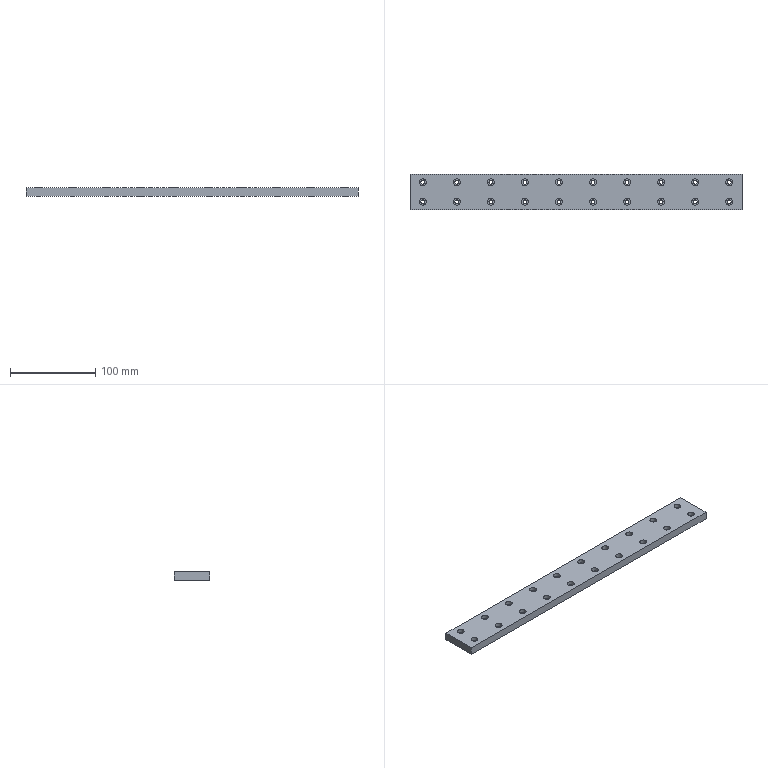Part | NX | features MGW_MGWR15R3900001 2 | 1 solid | 66 faces | box 390 x 42 x 9.5 mm | volume 149496 mm3 | cylinder 40 | plane 26 | commonest cylinder face diameters 4.5 x20 8 x20
STEP:
#1=CARTESIAN_POINT('',(182.25,13.5,0.));
#2=VERTEX_POINT('',#1);
#3=CARTESIAN_POINT('',(180.,13.5,0.));
#4=DIRECTION('',(0.,0.,1.));
#5=DIRECTION('',(1.,0.,0.));
#6=AXIS2_PLACEMENT_3D('',#3,#4,#5);
#7=CIRCLE('',#6,2.25);
#8=EDGE_CURVE('',#2,#2,#7,.T.);
#9=ORIENTED_EDGE('',*,*,#8,.F.);
#10=EDGE_LOOP('',(#9));
#11=FACE_BOUND('',#10,.T.);
#12=CARTESIAN_POINT('',(177.75,13.5,5.));
#13=VERTEX_POINT('',#12);
#14=CARTESIAN_POINT('',(180.,13.5,5.));
#15=DIRECTION('',(0.,0.,-1.));
#16=DIRECTION('',(-1.,0.,0.));
#17=AXIS2_PLACEMENT_3D('',#14,#15,#16);
#18=CIRCLE('',#17,2.25);
#19=EDGE_CURVE('',#13,#13,#18,.T.);
#20=ORIENTED_EDGE('',*,*,#19,.F.);
#21=EDGE_LOOP('',(#20));
#22=FACE_BOUND('',#21,.T.);
#23=CARTESIAN_POINT('',(180.,13.5,0.));
#24=DIRECTION('',(0.,0.,1.));
#25=DIRECTION('',(1.,0.,0.));
#26=AXIS2_PLACEMENT_3D('',#23,#24,#25);
#27=CYLINDRICAL_SURFACE('',#26,2.25);
#28=ADVANCED_FACE('',(#11,#22),#27,.F.);
#29=ORIENTED_EDGE('',*,*,#19,.T.);
#30=EDGE_LOOP('',(#29));
#31=FACE_BOUND('',#30,.T.);
#32=CARTESIAN_POINT('',(184.,13.5,5.));
#33=VERTEX_POINT('',#32);
#34=CARTESIAN_POINT('',(180.,13.5,5.));
#35=DIRECTION('',(0.,0.,1.));
#36=DIRECTION('',(1.,0.,0.));
#37=AXIS2_PLACEMENT_3D('',#34,#35,#36);
#38=CIRCLE('',#37,4.);
#39=EDGE_CURVE('',#33,#33,#38,.T.);
#40=ORIENTED_EDGE('',*,*,#39,.T.);
#41=EDGE_LOOP('',(#40));
#42=FACE_BOUND('',#41,.T.);
#43=CARTESIAN_POINT('',(180.,13.5,5.));
#44=DIRECTION('',(0.,0.,1.));
#45=DIRECTION('',(1.,0.,0.));
#46=AXIS2_PLACEMENT_3D('',#43,#44,#45);
#47=PLANE('',#46);
#48=ADVANCED_FACE('',(#31,#42),#47,.T.);
#49=ORIENTED_EDGE('',*,*,#39,.F.);
#50=EDGE_LOOP('',(#49));
#51=FACE_BOUND('',#50,.T.);
#52=CARTESIAN_POINT('',(176.,13.5,9.5));
#53=VERTEX_POINT('',#52);
#54=CARTESIAN_POINT('',(180.,13.5,9.5));
#55=DIRECTION('',(0.,0.,-1.));
#56=DIRECTION('',(-1.,0.,0.));
#57=AXIS2_PLACEMENT_3D('',#54,#55,#56);
#58=CIRCLE('',#57,4.);
#59=EDGE_CURVE('',#53,#53,#58,.T.);
#60=ORIENTED_EDGE('',*,*,#59,.F.);
#61=EDGE_LOOP('',(#60));
#62=FACE_BOUND('',#61,.T.);
#63=CARTESIAN_POINT('',(180.,13.5,5.));
#64=DIRECTION('',(0.,0.,1.));
#65=DIRECTION('',(1.,0.,0.));
#66=AXIS2_PLACEMENT_3D('',#63,#64,#65);
#67=CYLINDRICAL_SURFACE('',#66,4.);
#68=ADVANCED_FACE('',(#51,#62),#67,.F.);
#69=CARTESIAN_POINT('',(142.25,13.5,0.));
#70=VERTEX_POINT('',#69);
#71=CARTESIAN_POINT('',(140.,13.5,0.));
#72=DIRECTION('',(0.,0.,1.));
#73=DIRECTION('',(1.,0.,0.));
#74=AXIS2_PLACEMENT_3D('',#71,#72,#73);
#75=CIRCLE('',#74,2.25);
#76=EDGE_CURVE('',#70,#70,#75,.T.);
#77=ORIENTED_EDGE('',*,*,#76,.F.);
#78=EDGE_LOOP('',(#77));
#79=FACE_BOUND('',#78,.T.);
#80=CARTESIAN_POINT('',(137.75,13.5,5.));
#81=VERTEX_POINT('',#80);
#82=CARTESIAN_POINT('',(140.,13.5,5.));
#83=DIRECTION('',(0.,0.,-1.));
#84=DIRECTION('',(-1.,0.,0.));
#85=AXIS2_PLACEMENT_3D('',#82,#83,#84);
#86=CIRCLE('',#85,2.25);
#87=EDGE_CURVE('',#81,#81,#86,.T.);
#88=ORIENTED_EDGE('',*,*,#87,.F.);
#89=EDGE_LOOP('',(#88));
#90=FACE_BOUND('',#89,.T.);
#91=CARTESIAN_POINT('',(140.,13.5,0.));
#92=DIRECTION('',(0.,0.,1.));
#93=DIRECTION('',(1.,0.,0.));
#94=AXIS2_PLACEMENT_3D('',#91,#92,#93);
#95=CYLINDRICAL_SURFACE('',#94,2.25);
#96=ADVANCED_FACE('',(#79,#90),#95,.F.);
#97=ORIENTED_EDGE('',*,*,#87,.T.);
#98=EDGE_LOOP('',(#97));
#99=FACE_BOUND('',#98,.T.);
#100=CARTESIAN_POINT('',(144.,13.5,5.));
#101=VERTEX_POINT('',#100);
#102=CARTESIAN_POINT('',(140.,13.5,5.));
#103=DIRECTION('',(0.,0.,1.));
#104=DIRECTION('',(1.,0.,0.));
#105=AXIS2_PLACEMENT_3D('',#102,#103,#104);
#106=CIRCLE('',#105,4.);
#107=EDGE_CURVE('',#101,#101,#106,.T.);
#108=ORIENTED_EDGE('',*,*,#107,.T.);
#109=EDGE_LOOP('',(#108));
#110=FACE_BOUND('',#109,.T.);
#111=CARTESIAN_POINT('',(140.,13.5,5.));
#112=DIRECTION('',(0.,0.,1.));
#113=DIRECTION('',(1.,0.,0.));
#114=AXIS2_PLACEMENT_3D('',#111,#112,#113);
#115=PLANE('',#114);
#116=ADVANCED_FACE('',(#99,#110),#115,.T.);
#117=CARTESIAN_POINT('',(136.,13.5,9.5));
#118=VERTEX_POINT('',#117);
#119=CARTESIAN_POINT('',(140.,13.5,9.5));
#120=DIRECTION('',(0.,0.,-1.));
#121=DIRECTION('',(-1.,0.,0.));
#122=AXIS2_PLACEMENT_3D('',#119,#120,#121);
#123=CIRCLE('',#122,4.);
#124=EDGE_CURVE('',#118,#118,#123,.T.);
#125=ORIENTED_EDGE('',*,*,#124,.F.);
#126=EDGE_LOOP('',(#125));
#127=FACE_BOUND('',#126,.T.);
#128=ORIENTED_EDGE('',*,*,#107,.F.);
#129=EDGE_LOOP('',(#128));
#130=FACE_BOUND('',#129,.T.);
#131=CARTESIAN_POINT('',(140.,13.5,5.));
#132=DIRECTION('',(0.,0.,1.));
#133=DIRECTION('',(1.,0.,0.));
#134=AXIS2_PLACEMENT_3D('',#131,#132,#133);
#135=CYLINDRICAL_SURFACE('',#134,4.);
#136=ADVANCED_FACE('',(#127,#130),#135,.F.);
#137=CARTESIAN_POINT('',(97.75,13.5,5.));
#138=VERTEX_POINT('',#137);
#139=CARTESIAN_POINT('',(100.,13.5,5.));
#140=DIRECTION('',(0.,0.,-1.));
#141=DIRECTION('',(-1.,0.,0.));
#142=AXIS2_PLACEMENT_3D('',#139,#140,#141);
#143=CIRCLE('',#142,2.25);
#144=EDGE_CURVE('',#138,#138,#143,.T.);
#145=ORIENTED_EDGE('',*,*,#144,.F.);
#146=EDGE_LOOP('',(#145));
#147=FACE_BOUND('',#146,.T.);
#148=CARTESIAN_POINT('',(102.25,13.5,0.));
#149=VERTEX_POINT('',#148);
#150=CARTESIAN_POINT('',(100.,13.5,0.));
#151=DIRECTION('',(0.,0.,1.));
#152=DIRECTION('',(1.,0.,0.));
#153=AXIS2_PLACEMENT_3D('',#150,#151,#152);
#154=CIRCLE('',#153,2.25);
#155=EDGE_CURVE('',#149,#149,#154,.T.);
#156=ORIENTED_EDGE('',*,*,#155,.F.);
#157=EDGE_LOOP('',(#156));
#158=FACE_BOUND('',#157,.T.);
#159=CARTESIAN_POINT('',(100.,13.5,0.));
#160=DIRECTION('',(0.,0.,1.));
#161=DIRECTION('',(1.,0.,0.));
#162=AXIS2_PLACEMENT_3D('',#159,#160,#161);
#163=CYLINDRICAL_SURFACE('',#162,2.25);
#164=ADVANCED_FACE('',(#147,#158),#163,.F.);
#165=ORIENTED_EDGE('',*,*,#144,.T.);
#166=EDGE_LOOP('',(#165));
#167=FACE_BOUND('',#166,.T.);
#168=CARTESIAN_POINT('',(104.,13.5,5.));
#169=VERTEX_POINT('',#168);
#170=CARTESIAN_POINT('',(100.,13.5,5.));
#171=DIRECTION('',(0.,0.,1.));
#172=DIRECTION('',(1.,0.,0.));
#173=AXIS2_PLACEMENT_3D('',#170,#171,#172);
#174=CIRCLE('',#173,4.);
#175=EDGE_CURVE('',#169,#169,#174,.T.);
#176=ORIENTED_EDGE('',*,*,#175,.T.);
#177=EDGE_LOOP('',(#176));
#178=FACE_BOUND('',#177,.T.);
#179=CARTESIAN_POINT('',(100.,13.5,5.));
#180=DIRECTION('',(0.,0.,1.));
#181=DIRECTION('',(1.,0.,0.));
#182=AXIS2_PLACEMENT_3D('',#179,#180,#181);
#183=PLANE('',#182);
#184=ADVANCED_FACE('',(#167,#178),#183,.T.);
#185=CARTESIAN_POINT('',(96.,13.5,9.5));
#186=VERTEX_POINT('',#185);
#187=CARTESIAN_POINT('',(100.,13.5,9.5));
#188=DIRECTION('',(0.,0.,-1.));
#189=DIRECTION('',(-1.,0.,0.));
#190=AXIS2_PLACEMENT_3D('',#187,#188,#189);
#191=CIRCLE('',#190,4.);
#192=EDGE_CURVE('',#186,#186,#191,.T.);
#193=ORIENTED_EDGE('',*,*,#192,.F.);
#194=EDGE_LOOP('',(#193));
#195=FACE_BOUND('',#194,.T.);
#196=ORIENTED_EDGE('',*,*,#175,.F.);
#197=EDGE_LOOP('',(#196));
#198=FACE_BOUND('',#197,.T.);
#199=CARTESIAN_POINT('',(100.,13.5,5.));
#200=DIRECTION('',(0.,0.,1.));
#201=DIRECTION('',(1.,0.,0.));
#202=AXIS2_PLACEMENT_3D('',#199,#200,#201);
#203=CYLINDRICAL_SURFACE('',#202,4.);
#204=ADVANCED_FACE('',(#195,#198),#203,.F.);
#205=CARTESIAN_POINT('',(62.25,13.5,0.));
#206=VERTEX_POINT('',#205);
#207=CARTESIAN_POINT('',(60.,13.5,0.));
#208=DIRECTION('',(0.,0.,1.));
#209=DIRECTION('',(1.,0.,0.));
#210=AXIS2_PLACEMENT_3D('',#207,#208,#209);
#211=CIRCLE('',#210,2.25);
#212=EDGE_CURVE('',#206,#206,#211,.T.);
#213=ORIENTED_EDGE('',*,*,#212,.F.);
#214=EDGE_LOOP('',(#213));
#215=FACE_BOUND('',#214,.T.);
#216=CARTESIAN_POINT('',(57.75,13.5,5.));
#217=VERTEX_POINT('',#216);
#218=CARTESIAN_POINT('',(60.,13.5,5.));
#219=DIRECTION('',(0.,0.,-1.));
#220=DIRECTION('',(-1.,0.,0.));
#221=AXIS2_PLACEMENT_3D('',#218,#219,#220);
#222=CIRCLE('',#221,2.25);
#223=EDGE_CURVE('',#217,#217,#222,.T.);
#224=ORIENTED_EDGE('',*,*,#223,.F.);
#225=EDGE_LOOP('',(#224));
#226=FACE_BOUND('',#225,.T.);
#227=CARTESIAN_POINT('',(60.,13.5,0.));
#228=DIRECTION('',(0.,0.,1.));
#229=DIRECTION('',(1.,0.,0.));
#230=AXIS2_PLACEMENT_3D('',#227,#228,#229);
#231=CYLINDRICAL_SURFACE('',#230,2.25);
#232=ADVANCED_FACE('',(#215,#226),#231,.F.);
#233=ORIENTED_EDGE('',*,*,#223,.T.);
#234=EDGE_LOOP('',(#233));
#235=FACE_BOUND('',#234,.T.);
#236=CARTESIAN_POINT('',(64.,13.5,5.));
#237=VERTEX_POINT('',#236);
#238=CARTESIAN_POINT('',(60.,13.5,5.));
#239=DIRECTION('',(0.,0.,1.));
#240=DIRECTION('',(1.,0.,0.));
#241=AXIS2_PLACEMENT_3D('',#238,#239,#240);
#242=CIRCLE('',#241,4.);
#243=EDGE_CURVE('',#237,#237,#242,.T.);
#244=ORIENTED_EDGE('',*,*,#243,.T.);
#245=EDGE_LOOP('',(#244));
#246=FACE_BOUND('',#245,.T.);
#247=CARTESIAN_POINT('',(60.,13.5,5.));
#248=DIRECTION('',(0.,0.,1.));
#249=DIRECTION('',(1.,0.,0.));
#250=AXIS2_PLACEMENT_3D('',#247,#248,#249);
#251=PLANE('',#250);
#252=ADVANCED_FACE('',(#235,#246),#251,.T.);
#253=CARTESIAN_POINT('',(56.,13.5,9.5));
#254=VERTEX_POINT('',#253);
#255=CARTESIAN_POINT('',(60.,13.5,9.5));
#256=DIRECTION('',(0.,0.,-1.));
#257=DIRECTION('',(-1.,0.,0.));
#258=AXIS2_PLACEMENT_3D('',#255,#256,#257);
#259=CIRCLE('',#258,4.);
#260=EDGE_CURVE('',#254,#254,#259,.T.);
#261=ORIENTED_EDGE('',*,*,#260,.F.);
#262=EDGE_LOOP('',(#261));
#263=FACE_BOUND('',#262,.T.);
#264=ORIENTED_EDGE('',*,*,#243,.F.);
#265=EDGE_LOOP('',(#264));
#266=FACE_BOUND('',#265,.T.);
#267=CARTESIAN_POINT('',(60.,13.5,5.));
#268=DIRECTION('',(0.,0.,1.));
#269=DIRECTION('',(1.,0.,0.));
#270=AXIS2_PLACEMENT_3D('',#267,#268,#269);
#271=CYLINDRICAL_SURFACE('',#270,4.);
#272=ADVANCED_FACE('',(#263,#266),#271,.F.);
#273=CARTESIAN_POINT('',(17.75,13.5,5.));
#274=VERTEX_POINT('',#273);
#275=CARTESIAN_POINT('',(20.,13.5,5.));
#276=DIRECTION('',(0.,0.,-1.));
#277=DIRECTION('',(-1.,0.,0.));
#278=AXIS2_PLACEMENT_3D('',#275,#276,#277);
#279=CIRCLE('',#278,2.25);
#280=EDGE_CURVE('',#274,#274,#279,.T.);
#281=ORIENTED_EDGE('',*,*,#280,.F.);
#282=EDGE_LOOP('',(#281));
#283=FACE_BOUND('',#282,.T.);
#284=CARTESIAN_POINT('',(22.25,13.5,0.));
#285=VERTEX_POINT('',#284);
#286=CARTESIAN_POINT('',(20.,13.5,0.));
#287=DIRECTION('',(0.,0.,1.));
#288=DIRECTION('',(1.,0.,0.));
#289=AXIS2_PLACEMENT_3D('',#286,#287,#288);
#290=CIRCLE('',#289,2.25);
#291=EDGE_CURVE('',#285,#285,#290,.T.);
#292=ORIENTED_EDGE('',*,*,#291,.F.);
#293=EDGE_LOOP('',(#292));
#294=FACE_BOUND('',#293,.T.);
#295=CARTESIAN_POINT('',(20.,13.5,0.));
#296=DIRECTION('',(0.,0.,1.));
#297=DIRECTION('',(1.,0.,0.));
#298=AXIS2_PLACEMENT_3D('',#295,#296,#297);
#299=CYLINDRICAL_SURFACE('',#298,2.25);
#300=ADVANCED_FACE('',(#283,#294),#299,.F.);
#301=ORIENTED_EDGE('',*,*,#280,.T.);
#302=EDGE_LOOP('',(#301));
#303=FACE_BOUND('',#302,.T.);
#304=CARTESIAN_POINT('',(24.,13.5,5.));
#305=VERTEX_POINT('',#304);
#306=CARTESIAN_POINT('',(20.,13.5,5.));
#307=DIRECTION('',(0.,0.,1.));
#308=DIRECTION('',(1.,0.,0.));
#309=AXIS2_PLACEMENT_3D('',#306,#307,#308);
#310=CIRCLE('',#309,4.);
#311=EDGE_CURVE('',#305,#305,#310,.T.);
#312=ORIENTED_EDGE('',*,*,#311,.T.);
#313=EDGE_LOOP('',(#312));
#314=FACE_BOUND('',#313,.T.);
#315=CARTESIAN_POINT('',(20.,13.5,5.));
#316=DIRECTION('',(0.,0.,1.));
#317=DIRECTION('',(1.,0.,0.));
#318=AXIS2_PLACEMENT_3D('',#315,#316,#317);
#319=PLANE('',#318);
#320=ADVANCED_FACE('',(#303,#314),#319,.T.);
#321=ORIENTED_EDGE('',*,*,#311,.F.);
#322=EDGE_LOOP('',(#321));
#323=FACE_BOUND('',#322,.T.);
#324=CARTESIAN_POINT('',(16.,13.5,9.5));
#325=VERTEX_POINT('',#324);
#326=CARTESIAN_POINT('',(20.,13.5,9.5));
#327=DIRECTION('',(0.,0.,-1.));
#328=DIRECTION('',(-1.,0.,0.));
#329=AXIS2_PLACEMENT_3D('',#326,#327,#328);
#330=CIRCLE('',#329,4.);
#331=EDGE_CURVE('',#325,#325,#330,.T.);
#332=ORIENTED_EDGE('',*,*,#331,.F.);
#333=EDGE_LOOP('',(#332));
#334=FACE_BOUND('',#333,.T.);
#335=CARTESIAN_POINT('',(20.,13.5,5.));
#336=DIRECTION('',(0.,0.,1.));
#337=DIRECTION('',(1.,0.,0.));
#338=AXIS2_PLACEMENT_3D('',#335,#336,#337);
#339=CYLINDRICAL_SURFACE('',#338,4.);
#340=ADVANCED_FACE('',(#323,#334),#339,.F.);
#341=CARTESIAN_POINT('',(-22.25,13.5,5.));
#342=VERTEX_POINT('',#341);
#343=CARTESIAN_POINT('',(-20.,13.5,5.));
#344=DIRECTION('',(0.,0.,-1.));
#345=DIRECTION('',(-1.,0.,0.));
#346=AXIS2_PLACEMENT_3D('',#343,#344,#345);
#347=CIRCLE('',#346,2.25);
#348=EDGE_CURVE('',#342,#342,#347,.T.);
#349=ORIENTED_EDGE('',*,*,#348,.F.);
#350=EDGE_LOOP('',(#349));
#351=FACE_BOUND('',#350,.T.);
#352=CARTESIAN_POINT('',(-17.75,13.5,0.));
#353=VERTEX_POINT('',#352);
#354=CARTESIAN_POINT('',(-20.,13.5,0.));
#355=DIRECTION('',(0.,0.,1.));
#356=DIRECTION('',(1.,0.,0.));
#357=AXIS2_PLACEMENT_3D('',#354,#355,#356);
#358=CIRCLE('',#357,2.25);
#359=EDGE_CURVE('',#353,#353,#358,.T.);
#360=ORIENTED_EDGE('',*,*,#359,.F.);
#361=EDGE_LOOP('',(#360));
#362=FACE_BOUND('',#361,.T.);
#363=CARTESIAN_POINT('',(-20.,13.5,0.));
#364=DIRECTION('',(0.,0.,1.));
#365=DIRECTION('',(1.,0.,0.));
#366=AXIS2_PLACEMENT_3D('',#363,#364,#365);
#367=CYLINDRICAL_SURFACE('',#366,2.25);
#368=ADVANCED_FACE('',(#351,#362),#367,.F.);
#369=ORIENTED_EDGE('',*,*,#348,.T.);
#370=EDGE_LOOP('',(#369));
#371=FACE_BOUND('',#370,.T.);
#372=CARTESIAN_POINT('',(-16.,13.5,5.));
#373=VERTEX_POINT('',#372);
#374=CARTESIAN_POINT('',(-20.,13.5,5.));
#375=DIRECTION('',(0.,0.,1.));
#376=DIRECTION('',(1.,0.,0.));
#377=AXIS2_PLACEMENT_3D('',#374,#375,#376);
#378=CIRCLE('',#377,4.);
#379=EDGE_CURVE('',#373,#373,#378,.T.);
#380=ORIENTED_EDGE('',*,*,#379,.T.);
#381=EDGE_LOOP('',(#380));
#382=FACE_BOUND('',#381,.T.);
#383=CARTESIAN_POINT('',(-20.,13.5,5.));
#384=DIRECTION('',(0.,0.,1.));
#385=DIRECTION('',(1.,0.,0.));
#386=AXIS2_PLACEMENT_3D('',#383,#384,#385);
#387=PLANE('',#386);
#388=ADVANCED_FACE('',(#371,#382),#387,.T.);
#389=CARTESIAN_POINT('',(-24.,13.5,9.5));
#390=VERTEX_POINT('',#389);
#391=CARTESIAN_POINT('',(-20.,13.5,9.5));
#392=DIRECTION('',(0.,0.,-1.));
#393=DIRECTION('',(-1.,0.,0.));
#394=AXIS2_PLACEMENT_3D('',#391,#392,#393);
#395=CIRCLE('',#394,4.);
#396=EDGE_CURVE('',#390,#390,#395,.T.);
#397=ORIENTED_EDGE('',*,*,#396,.F.);
#398=EDGE_LOOP('',(#397));
#399=FACE_BOUND('',#398,.T.);
#400=ORIENTED_EDGE('',*,*,#379,.F.);
#401=EDGE_LOOP('',(#400));
#402=FACE_BOUND('',#401,.T.);
#403=CARTESIAN_POINT('',(-20.,13.5,5.));
#404=DIRECTION('',(0.,0.,1.));
#405=DIRECTION('',(1.,0.,0.));
#406=AXIS2_PLACEMENT_3D('',#403,#404,#405);
#407=CYLINDRICAL_SURFACE('',#406,4.);
#408=ADVANCED_FACE('',(#399,#402),#407,.F.);
#409=CARTESIAN_POINT('',(-57.75,13.5,0.));
#410=VERTEX_POINT('',#409);
#411=CARTESIAN_POINT('',(-60.,13.5,0.));
#412=DIRECTION('',(0.,0.,1.));
#413=DIRECTION('',(1.,0.,0.));
#414=AXIS2_PLACEMENT_3D('',#411,#412,#413);
#415=CIRCLE('',#414,2.25);
#416=EDGE_CURVE('',#410,#410,#415,.T.);
#417=ORIENTED_EDGE('',*,*,#416,.F.);
#418=EDGE_LOOP('',(#417));
#419=FACE_BOUND('',#418,.T.);
#420=CARTESIAN_POINT('',(-62.25,13.5,5.));
#421=VERTEX_POINT('',#420);
#422=CARTESIAN_POINT('',(-60.,13.5,5.));
#423=DIRECTION('',(0.,0.,-1.));
#424=DIRECTION('',(-1.,0.,0.));
#425=AXIS2_PLACEMENT_3D('',#422,#423,#424);
#426=CIRCLE('',#425,2.25);
#427=EDGE_CURVE('',#421,#421,#426,.T.);
#428=ORIENTED_EDGE('',*,*,#427,.F.);
#429=EDGE_LOOP('',(#428));
#430=FACE_BOUND('',#429,.T.);
#431=CARTESIAN_POINT('',(-60.,13.5,0.));
#432=DIRECTION('',(0.,0.,1.));
#433=DIRECTION('',(1.,0.,0.));
#434=AXIS2_PLACEMENT_3D('',#431,#432,#433);
#435=CYLINDRICAL_SURFACE('',#434,2.25);
#436=ADVANCED_FACE('',(#419,#430),#435,.F.);
#437=ORIENTED_EDGE('',*,*,#427,.T.);
#438=EDGE_LOOP('',(#437));
#439=FACE_BOUND('',#438,.T.);
#440=CARTESIAN_POINT('',(-56.,13.5,5.));
#441=VERTEX_POINT('',#440);
#442=CARTESIAN_POINT('',(-60.,13.5,5.));
#443=DIRECTION('',(0.,0.,1.));
#444=DIRECTION('',(1.,0.,0.));
#445=AXIS2_PLACEMENT_3D('',#442,#443,#444);
#446=CIRCLE('',#445,4.);
#447=EDGE_CURVE('',#441,#441,#446,.T.);
#448=ORIENTED_EDGE('',*,*,#447,.T.);
#449=EDGE_LOOP('',(#448));
#450=FACE_BOUND('',#449,.T.);
#451=CARTESIAN_POINT('',(-60.,13.5,5.));
#452=DIRECTION('',(0.,0.,1.));
#453=DIRECTION('',(1.,0.,0.));
#454=AXIS2_PLACEMENT_3D('',#451,#452,#453);
#455=PLANE('',#454);
#456=ADVANCED_FACE('',(#439,#450),#455,.T.);
#457=CARTESIAN_POINT('',(-64.,13.5,9.5));
#458=VERTEX_POINT('',#457);
#459=CARTESIAN_POINT('',(-60.,13.5,9.5));
#460=DIRECTION('',(0.,0.,-1.));
#461=DIRECTION('',(-1.,0.,0.));
#462=AXIS2_PLACEMENT_3D('',#459,#460,#461);
#463=CIRCLE('',#462,4.);
#464=EDGE_CURVE('',#458,#458,#463,.T.);
#465=ORIENTED_EDGE('',*,*,#464,.F.);
#466=EDGE_LOOP('',(#465));
#467=FACE_BOUND('',#466,.T.);
#468=ORIENTED_EDGE('',*,*,#447,.F.);
#469=EDGE_LOOP('',(#468));
#470=FACE_BOUND('',#469,.T.);
#471=CARTESIAN_POINT('',(-60.,13.5,5.));
#472=DIRECTION('',(0.,0.,1.));
#473=DIRECTION('',(1.,0.,0.));
#474=AXIS2_PLACEMENT_3D('',#471,#472,#473);
#475=CYLINDRICAL_SURFACE('',#474,4.);
#476=ADVANCED_FACE('',(#467,#470),#475,.F.);
#477=CARTESIAN_POINT('',(-102.25,13.5,5.));
#478=VERTEX_POINT('',#477);
#479=CARTESIAN_POINT('',(-100.,13.5,5.));
#480=DIRECTION('',(0.,0.,-1.));
#481=DIRECTION('',(-1.,0.,0.));
#482=AXIS2_PLACEMENT_3D('',#479,#480,#481);
#483=CIRCLE('',#482,2.25);
#484=EDGE_CURVE('',#478,#478,#483,.T.);
#485=ORIENTED_EDGE('',*,*,#484,.F.);
#486=EDGE_LOOP('',(#485));
#487=FACE_BOUND('',#486,.T.);
#488=CARTESIAN_POINT('',(-97.75,13.5,0.));
#489=VERTEX_POINT('',#488);
#490=CARTESIAN_POINT('',(-100.,13.5,0.));
#491=DIRECTION('',(0.,0.,1.));
#492=DIRECTION('',(1.,0.,0.));
#493=AXIS2_PLACEMENT_3D('',#490,#491,#492);
#494=CIRCLE('',#493,2.25);
#495=EDGE_CURVE('',#489,#489,#494,.T.);
#496=ORIENTED_EDGE('',*,*,#495,.F.);
#497=EDGE_LOOP('',(#496));
#498=FACE_BOUND('',#497,.T.);
#499=CARTESIAN_POINT('',(-100.,13.5,0.));
#500=DIRECTION('',(0.,0.,1.));
#501=DIRECTION('',(1.,0.,0.));
#502=AXIS2_PLACEMENT_3D('',#499,#500,#501);
#503=CYLINDRICAL_SURFACE('',#502,2.25);
#504=ADVANCED_FACE('',(#487,#498),#503,.F.);
#505=ORIENTED_EDGE('',*,*,#484,.T.);
#506=EDGE_LOOP('',(#505));
#507=FACE_BOUND('',#506,.T.);
#508=CARTESIAN_POINT('',(-96.,13.5,5.));
#509=VERTEX_POINT('',#508);
#510=CARTESIAN_POINT('',(-100.,13.5,5.));
#511=DIRECTION('',(0.,0.,1.));
#512=DIRECTION('',(1.,0.,0.));
#513=AXIS2_PLACEMENT_3D('',#510,#511,#512);
#514=CIRCLE('',#513,4.);
#515=EDGE_CURVE('',#509,#509,#514,.T.);
#516=ORIENTED_EDGE('',*,*,#515,.T.);
#517=EDGE_LOOP('',(#516));
#518=FACE_BOUND('',#517,.T.);
#519=CARTESIAN_POINT('',(-100.,13.5,5.));
#520=DIRECTION('',(0.,0.,1.));
#521=DIRECTION('',(1.,0.,0.));
#522=AXIS2_PLACEMENT_3D('',#519,#520,#521);
#523=PLANE('',#522);
#524=ADVANCED_FACE('',(#507,#518),#523,.T.);
#525=ORIENTED_EDGE('',*,*,#515,.F.);
#526=EDGE_LOOP('',(#525));
#527=FACE_BOUND('',#526,.T.);
#528=CARTESIAN_POINT('',(-104.,13.5,9.5));
#529=VERTEX_POINT('',#528);
#530=CARTESIAN_POINT('',(-100.,13.5,9.5));
#531=DIRECTION('',(0.,0.,-1.));
#532=DIRECTION('',(-1.,0.,0.));
#533=AXIS2_PLACEMENT_3D('',#530,#531,#532);
#534=CIRCLE('',#533,4.);
#535=EDGE_CURVE('',#529,#529,#534,.T.);
#536=ORIENTED_EDGE('',*,*,#535,.F.);
#537=EDGE_LOOP('',(#536));
#538=FACE_BOUND('',#537,.T.);
#539=CARTESIAN_POINT('',(-100.,13.5,5.));
#540=DIRECTION('',(0.,0.,1.));
#541=DIRECTION('',(1.,0.,0.));
#542=AXIS2_PLACEMENT_3D('',#539,#540,#541);
#543=CYLINDRICAL_SURFACE('',#542,4.);
#544=ADVANCED_FACE('',(#527,#538),#543,.F.);
#545=CARTESIAN_POINT('',(182.25,36.5,5.));
#546=VERTEX_POINT('',#545);
#547=CARTESIAN_POINT('',(180.,36.5,5.));
#548=DIRECTION('',(0.,0.,-1.));
#549=DIRECTION('',(1.,0.,0.));
#550=AXIS2_PLACEMENT_3D('',#547,#548,#549);
#551=CIRCLE('',#550,2.25);
#552=EDGE_CURVE('',#546,#546,#551,.T.);
#553=ORIENTED_EDGE('',*,*,#552,.T.);
#554=EDGE_LOOP('',(#553));
#555=FACE_BOUND('',#554,.T.);
#556=CARTESIAN_POINT('',(184.,36.5,5.));
#557=VERTEX_POINT('',#556);
#558=CARTESIAN_POINT('',(180.,36.5,5.));
#559=DIRECTION('',(0.,0.,1.));
#560=DIRECTION('',(1.,0.,0.));
#561=AXIS2_PLACEMENT_3D('',#558,#559,#560);
#562=CIRCLE('',#561,4.);
#563=EDGE_CURVE('',#557,#557,#562,.T.);
#564=ORIENTED_EDGE('',*,*,#563,.T.);
#565=EDGE_LOOP('',(#564));
#566=FACE_BOUND('',#565,.T.);
#567=CARTESIAN_POINT('',(180.,36.5,5.));
#568=DIRECTION('',(0.,0.,1.));
#569=DIRECTION('',(1.,0.,0.));
#570=AXIS2_PLACEMENT_3D('',#567,#568,#569);
#571=PLANE('',#570);
#572=ADVANCED_FACE('',(#555,#566),#571,.T.);
#573=ORIENTED_EDGE('',*,*,#563,.F.);
#574=EDGE_LOOP('',(#573));
#575=FACE_BOUND('',#574,.T.);
#576=CARTESIAN_POINT('',(176.,36.5,9.5));
#577=VERTEX_POINT('',#576);
#578=CARTESIAN_POINT('',(180.,36.5,9.5));
#579=DIRECTION('',(0.,0.,-1.));
#580=DIRECTION('',(-1.,0.,0.));
#581=AXIS2_PLACEMENT_3D('',#578,#579,#580);
#582=CIRCLE('',#581,4.);
#583=EDGE_CURVE('',#577,#577,#582,.T.);
#584=ORIENTED_EDGE('',*,*,#583,.F.);
#585=EDGE_LOOP('',(#584));
#586=FACE_BOUND('',#585,.T.);
#587=CARTESIAN_POINT('',(180.,36.5,5.));
#588=DIRECTION('',(0.,0.,1.));
#589=DIRECTION('',(1.,0.,0.));
#590=AXIS2_PLACEMENT_3D('',#587,#588,#589);
#591=CYLINDRICAL_SURFACE('',#590,4.);
#592=ADVANCED_FACE('',(#575,#586),#591,.F.);
#593=CARTESIAN_POINT('',(137.75,36.5,5.));
#594=VERTEX_POINT('',#593);
#595=CARTESIAN_POINT('',(140.,36.5,5.));
#596=DIRECTION('',(0.,0.,-1.));
#597=DIRECTION('',(-1.,0.,0.));
#598=AXIS2_PLACEMENT_3D('',#595,#596,#597);
#599=CIRCLE('',#598,2.25);
#600=EDGE_CURVE('',#594,#594,#599,.T.);
#601=ORIENTED_EDGE('',*,*,#600,.F.);
#602=EDGE_LOOP('',(#601));
#603=FACE_BOUND('',#602,.T.);
#604=CARTESIAN_POINT('',(142.25,36.5,0.));
#605=VERTEX_POINT('',#604);
#606=CARTESIAN_POINT('',(140.,36.5,0.));
#607=DIRECTION('',(0.,0.,1.));
#608=DIRECTION('',(1.,0.,0.));
#609=AXIS2_PLACEMENT_3D('',#606,#607,#608);
#610=CIRCLE('',#609,2.25);
#611=EDGE_CURVE('',#605,#605,#610,.T.);
#612=ORIENTED_EDGE('',*,*,#611,.F.);
#613=EDGE_LOOP('',(#612));
#614=FACE_BOUND('',#613,.T.);
#615=CARTESIAN_POINT('',(140.,36.5,0.));
#616=DIRECTION('',(0.,0.,1.));
#617=DIRECTION('',(1.,0.,0.));
#618=AXIS2_PLACEMENT_3D('',#615,#616,#617);
#619=CYLINDRICAL_SURFACE('',#618,2.25);
#620=ADVANCED_FACE('',(#603,#614),#619,.F.);
#621=ORIENTED_EDGE('',*,*,#600,.T.);
#622=EDGE_LOOP('',(#621));
#623=FACE_BOUND('',#622,.T.);
#624=CARTESIAN_POINT('',(144.,36.5,5.));
#625=VERTEX_POINT('',#624);
#626=CARTESIAN_POINT('',(140.,36.5,5.));
#627=DIRECTION('',(0.,0.,1.));
#628=DIRECTION('',(1.,0.,0.));
#629=AXIS2_PLACEMENT_3D('',#626,#627,#628);
#630=CIRCLE('',#629,4.);
#631=EDGE_CURVE('',#625,#625,#630,.T.);
#632=ORIENTED_EDGE('',*,*,#631,.T.);
#633=EDGE_LOOP('',(#632));
#634=FACE_BOUND('',#633,.T.);
#635=CARTESIAN_POINT('',(140.,36.5,5.));
#636=DIRECTION('',(0.,0.,1.));
#637=DIRECTION('',(1.,0.,0.));
#638=AXIS2_PLACEMENT_3D('',#635,#636,#637);
#639=PLANE('',#638);
#640=ADVANCED_FACE('',(#623,#634),#639,.T.);
#641=CARTESIAN_POINT('',(136.,36.5,9.5));
#642=VERTEX_POINT('',#641);
#643=CARTESIAN_POINT('',(140.,36.5,9.5));
#644=DIRECTION('',(0.,0.,-1.));
#645=DIRECTION('',(-1.,0.,0.));
#646=AXIS2_PLACEMENT_3D('',#643,#644,#645);
#647=CIRCLE('',#646,4.);
#648=EDGE_CURVE('',#642,#642,#647,.T.);
#649=ORIENTED_EDGE('',*,*,#648,.F.);
#650=EDGE_LOOP('',(#649));
#651=FACE_BOUND('',#650,.T.);
#652=ORIENTED_EDGE('',*,*,#631,.F.);
#653=EDGE_LOOP('',(#652));
#654=FACE_BOUND('',#653,.T.);
#655=CARTESIAN_POINT('',(140.,36.5,5.));
#656=DIRECTION('',(0.,0.,1.));
#657=DIRECTION('',(1.,0.,0.));
#658=AXIS2_PLACEMENT_3D('',#655,#656,#657);
#659=CYLINDRICAL_SURFACE('',#658,4.);
#660=ADVANCED_FACE('',(#651,#654),#659,.F.);
#661=CARTESIAN_POINT('',(97.75,36.5,5.));
#662=VERTEX_POINT('',#661);
#663=CARTESIAN_POINT('',(100.,36.5,5.));
#664=DIRECTION('',(0.,0.,-1.));
#665=DIRECTION('',(-1.,0.,0.));
#666=AXIS2_PLACEMENT_3D('',#663,#664,#665);
#667=CIRCLE('',#666,2.25);
#668=EDGE_CURVE('',#662,#662,#667,.T.);
#669=ORIENTED_EDGE('',*,*,#668,.F.);
#670=EDGE_LOOP('',(#669));
#671=FACE_BOUND('',#670,.T.);
#672=CARTESIAN_POINT('',(102.25,36.5,0.));
#673=VERTEX_POINT('',#672);
#674=CARTESIAN_POINT('',(100.,36.5,0.));
#675=DIRECTION('',(0.,0.,1.));
#676=DIRECTION('',(1.,0.,0.));
#677=AXIS2_PLACEMENT_3D('',#674,#675,#676);
#678=CIRCLE('',#677,2.25);
#679=EDGE_CURVE('',#673,#673,#678,.T.);
#680=ORIENTED_EDGE('',*,*,#679,.F.);
#681=EDGE_LOOP('',(#680));
#682=FACE_BOUND('',#681,.T.);
#683=CARTESIAN_POINT('',(100.,36.5,0.));
#684=DIRECTION('',(0.,0.,1.));
#685=DIRECTION('',(1.,0.,0.));
#686=AXIS2_PLACEMENT_3D('',#683,#684,#685);
#687=CYLINDRICAL_SURFACE('',#686,2.25);
#688=ADVANCED_FACE('',(#671,#682),#687,.F.);
#689=ORIENTED_EDGE('',*,*,#668,.T.);
#690=EDGE_LOOP('',(#689));
#691=FACE_BOUND('',#690,.T.);
#692=CARTESIAN_POINT('',(104.,36.5,5.));
#693=VERTEX_POINT('',#692);
#694=CARTESIAN_POINT('',(100.,36.5,5.));
#695=DIRECTION('',(0.,0.,1.));
#696=DIRECTION('',(1.,0.,0.));
#697=AXIS2_PLACEMENT_3D('',#694,#695,#696);
#698=CIRCLE('',#697,4.);
#699=EDGE_CURVE('',#693,#693,#698,.T.);
#700=ORIENTED_EDGE('',*,*,#699,.T.);
#701=EDGE_LOOP('',(#700));
#702=FACE_BOUND('',#701,.T.);
#703=CARTESIAN_POINT('',(100.,36.5,5.));
#704=DIRECTION('',(0.,0.,1.));
#705=DIRECTION('',(1.,0.,0.));
#706=AXIS2_PLACEMENT_3D('',#703,#704,#705);
#707=PLANE('',#706);
#708=ADVANCED_FACE('',(#691,#702),#707,.T.);
#709=CARTESIAN_POINT('',(96.,36.5,9.5));
#710=VERTEX_POINT('',#709);
#711=CARTESIAN_POINT('',(100.,36.5,9.5));
#712=DIRECTION('',(0.,0.,-1.));
#713=DIRECTION('',(-1.,0.,0.));
#714=AXIS2_PLACEMENT_3D('',#711,#712,#713);
#715=CIRCLE('',#714,4.);
#716=EDGE_CURVE('',#710,#710,#715,.T.);
#717=ORIENTED_EDGE('',*,*,#716,.F.);
#718=EDGE_LOOP('',(#717));
#719=FACE_BOUND('',#718,.T.);
#720=ORIENTED_EDGE('',*,*,#699,.F.);
#721=EDGE_LOOP('',(#720));
#722=FACE_BOUND('',#721,.T.);
#723=CARTESIAN_POINT('',(100.,36.5,5.));
#724=DIRECTION('',(0.,0.,1.));
#725=DIRECTION('',(1.,0.,0.));
#726=AXIS2_PLACEMENT_3D('',#723,#724,#725);
#727=CYLINDRICAL_SURFACE('',#726,4.);
#728=ADVANCED_FACE('',(#719,#722),#727,.F.);
#729=CARTESIAN_POINT('',(62.25,36.5,0.));
#730=VERTEX_POINT('',#729);
#731=CARTESIAN_POINT('',(60.,36.5,0.));
#732=DIRECTION('',(0.,0.,1.));
#733=DIRECTION('',(1.,0.,0.));
#734=AXIS2_PLACEMENT_3D('',#731,#732,#733);
#735=CIRCLE('',#734,2.25);
#736=EDGE_CURVE('',#730,#730,#735,.T.);
#737=ORIENTED_EDGE('',*,*,#736,.F.);
#738=EDGE_LOOP('',(#737));
#739=FACE_BOUND('',#738,.T.);
#740=CARTESIAN_POINT('',(57.75,36.5,5.));
#741=VERTEX_POINT('',#740);
#742=CARTESIAN_POINT('',(60.,36.5,5.));
#743=DIRECTION('',(0.,0.,-1.));
#744=DIRECTION('',(-1.,0.,0.));
#745=AXIS2_PLACEMENT_3D('',#742,#743,#744);
#746=CIRCLE('',#745,2.25);
#747=EDGE_CURVE('',#741,#741,#746,.T.);
#748=ORIENTED_EDGE('',*,*,#747,.F.);
#749=EDGE_LOOP('',(#748));
#750=FACE_BOUND('',#749,.T.);
#751=CARTESIAN_POINT('',(60.,36.5,0.));
#752=DIRECTION('',(0.,0.,1.));
#753=DIRECTION('',(1.,0.,0.));
#754=AXIS2_PLACEMENT_3D('',#751,#752,#753);
#755=CYLINDRICAL_SURFACE('',#754,2.25);
#756=ADVANCED_FACE('',(#739,#750),#755,.F.);
#757=ORIENTED_EDGE('',*,*,#747,.T.);
#758=EDGE_LOOP('',(#757));
#759=FACE_BOUND('',#758,.T.);
#760=CARTESIAN_POINT('',(64.,36.5,5.));
#761=VERTEX_POINT('',#760);
#762=CARTESIAN_POINT('',(60.,36.5,5.));
#763=DIRECTION('',(0.,0.,1.));
#764=DIRECTION('',(1.,0.,0.));
#765=AXIS2_PLACEMENT_3D('',#762,#763,#764);
#766=CIRCLE('',#765,4.);
#767=EDGE_CURVE('',#761,#761,#766,.T.);
#768=ORIENTED_EDGE('',*,*,#767,.T.);
#769=EDGE_LOOP('',(#768));
#770=FACE_BOUND('',#769,.T.);
#771=CARTESIAN_POINT('',(60.,36.5,5.));
#772=DIRECTION('',(0.,0.,1.));
#773=DIRECTION('',(1.,0.,0.));
#774=AXIS2_PLACEMENT_3D('',#771,#772,#773);
#775=PLANE('',#774);
#776=ADVANCED_FACE('',(#759,#770),#775,.T.);
#777=CARTESIAN_POINT('',(56.,36.5,9.5));
#778=VERTEX_POINT('',#777);
#779=CARTESIAN_POINT('',(60.,36.5,9.5));
#780=DIRECTION('',(0.,0.,-1.));
#781=DIRECTION('',(-1.,0.,0.));
#782=AXIS2_PLACEMENT_3D('',#779,#780,#781);
#783=CIRCLE('',#782,4.);
#784=EDGE_CURVE('',#778,#778,#783,.T.);
#785=ORIENTED_EDGE('',*,*,#784,.F.);
#786=EDGE_LOOP('',(#785));
#787=FACE_BOUND('',#786,.T.);
#788=ORIENTED_EDGE('',*,*,#767,.F.);
#789=EDGE_LOOP('',(#788));
#790=FACE_BOUND('',#789,.T.);
#791=CARTESIAN_POINT('',(60.,36.5,5.));
#792=DIRECTION('',(0.,0.,1.));
#793=DIRECTION('',(1.,0.,0.));
#794=AXIS2_PLACEMENT_3D('',#791,#792,#793);
#795=CYLINDRICAL_SURFACE('',#794,4.);
#796=ADVANCED_FACE('',(#787,#790),#795,.F.);
#797=CARTESIAN_POINT('',(17.75,36.5,5.));
#798=VERTEX_POINT('',#797);
#799=CARTESIAN_POINT('',(20.,36.5,5.));
#800=DIRECTION('',(0.,0.,-1.));
#801=DIRECTION('',(-1.,0.,0.));
#802=AXIS2_PLACEMENT_3D('',#799,#800,#801);
#803=CIRCLE('',#802,2.25);
#804=EDGE_CURVE('',#798,#798,#803,.T.);
#805=ORIENTED_EDGE('',*,*,#804,.F.);
#806=EDGE_LOOP('',(#805));
#807=FACE_BOUND('',#806,.T.);
#808=CARTESIAN_POINT('',(22.25,36.5,0.));
#809=VERTEX_POINT('',#808);
#810=CARTESIAN_POINT('',(20.,36.5,0.));
#811=DIRECTION('',(0.,0.,1.));
#812=DIRECTION('',(1.,0.,0.));
#813=AXIS2_PLACEMENT_3D('',#810,#811,#812);
#814=CIRCLE('',#813,2.25);
#815=EDGE_CURVE('',#809,#809,#814,.T.);
#816=ORIENTED_EDGE('',*,*,#815,.F.);
#817=EDGE_LOOP('',(#816));
#818=FACE_BOUND('',#817,.T.);
#819=CARTESIAN_POINT('',(20.,36.5,0.));
#820=DIRECTION('',(0.,0.,1.));
#821=DIRECTION('',(1.,0.,0.));
#822=AXIS2_PLACEMENT_3D('',#819,#820,#821);
#823=CYLINDRICAL_SURFACE('',#822,2.25);
#824=ADVANCED_FACE('',(#807,#818),#823,.F.);
#825=ORIENTED_EDGE('',*,*,#804,.T.);
#826=EDGE_LOOP('',(#825));
#827=FACE_BOUND('',#826,.T.);
#828=CARTESIAN_POINT('',(24.,36.5,5.));
#829=VERTEX_POINT('',#828);
#830=CARTESIAN_POINT('',(20.,36.5,5.));
#831=DIRECTION('',(0.,0.,1.));
#832=DIRECTION('',(1.,0.,0.));
#833=AXIS2_PLACEMENT_3D('',#830,#831,#832);
#834=CIRCLE('',#833,4.);
#835=EDGE_CURVE('',#829,#829,#834,.T.);
#836=ORIENTED_EDGE('',*,*,#835,.T.);
#837=EDGE_LOOP('',(#836));
#838=FACE_BOUND('',#837,.T.);
#839=CARTESIAN_POINT('',(20.,36.5,5.));
#840=DIRECTION('',(0.,0.,1.));
#841=DIRECTION('',(1.,0.,0.));
#842=AXIS2_PLACEMENT_3D('',#839,#840,#841);
#843=PLANE('',#842);
#844=ADVANCED_FACE('',(#827,#838),#843,.T.);
#845=ORIENTED_EDGE('',*,*,#835,.F.);
#846=EDGE_LOOP('',(#845));
#847=FACE_BOUND('',#846,.T.);
#848=CARTESIAN_POINT('',(16.,36.5,9.5));
#849=VERTEX_POINT('',#848);
#850=CARTESIAN_POINT('',(20.,36.5,9.5));
#851=DIRECTION('',(0.,0.,-1.));
#852=DIRECTION('',(-1.,0.,0.));
#853=AXIS2_PLACEMENT_3D('',#850,#851,#852);
#854=CIRCLE('',#853,4.);
#855=EDGE_CURVE('',#849,#849,#854,.T.);
#856=ORIENTED_EDGE('',*,*,#855,.F.);
#857=EDGE_LOOP('',(#856));
#858=FACE_BOUND('',#857,.T.);
#859=CARTESIAN_POINT('',(20.,36.5,5.));
#860=DIRECTION('',(0.,0.,1.));
#861=DIRECTION('',(1.,0.,0.));
#862=AXIS2_PLACEMENT_3D('',#859,#860,#861);
#863=CYLINDRICAL_SURFACE('',#862,4.);
#864=ADVANCED_FACE('',(#847,#858),#863,.F.);
#865=CARTESIAN_POINT('',(-22.25,36.5,5.));
#866=VERTEX_POINT('',#865);
#867=CARTESIAN_POINT('',(-20.,36.5,5.));
#868=DIRECTION('',(0.,0.,-1.));
#869=DIRECTION('',(-1.,0.,0.));
#870=AXIS2_PLACEMENT_3D('',#867,#868,#869);
#871=CIRCLE('',#870,2.25);
#872=EDGE_CURVE('',#866,#866,#871,.T.);
#873=ORIENTED_EDGE('',*,*,#872,.F.);
#874=EDGE_LOOP('',(#873));
#875=FACE_BOUND('',#874,.T.);
#876=CARTESIAN_POINT('',(-17.75,36.5,0.));
#877=VERTEX_POINT('',#876);
#878=CARTESIAN_POINT('',(-20.,36.5,0.));
#879=DIRECTION('',(0.,0.,1.));
#880=DIRECTION('',(1.,0.,0.));
#881=AXIS2_PLACEMENT_3D('',#878,#879,#880);
#882=CIRCLE('',#881,2.25);
#883=EDGE_CURVE('',#877,#877,#882,.T.);
#884=ORIENTED_EDGE('',*,*,#883,.F.);
#885=EDGE_LOOP('',(#884));
#886=FACE_BOUND('',#885,.T.);
#887=CARTESIAN_POINT('',(-20.,36.5,0.));
#888=DIRECTION('',(0.,0.,1.));
#889=DIRECTION('',(1.,0.,0.));
#890=AXIS2_PLACEMENT_3D('',#887,#888,#889);
#891=CYLINDRICAL_SURFACE('',#890,2.25);
#892=ADVANCED_FACE('',(#875,#886),#891,.F.);
#893=ORIENTED_EDGE('',*,*,#872,.T.);
#894=EDGE_LOOP('',(#893));
#895=FACE_BOUND('',#894,.T.);
#896=CARTESIAN_POINT('',(-16.,36.5,5.));
#897=VERTEX_POINT('',#896);
#898=CARTESIAN_POINT('',(-20.,36.5,5.));
#899=DIRECTION('',(0.,0.,1.));
#900=DIRECTION('',(1.,0.,0.));
#901=AXIS2_PLACEMENT_3D('',#898,#899,#900);
#902=CIRCLE('',#901,4.);
#903=EDGE_CURVE('',#897,#897,#902,.T.);
#904=ORIENTED_EDGE('',*,*,#903,.T.);
#905=EDGE_LOOP('',(#904));
#906=FACE_BOUND('',#905,.T.);
#907=CARTESIAN_POINT('',(-20.,36.5,5.));
#908=DIRECTION('',(0.,0.,1.));
#909=DIRECTION('',(1.,0.,0.));
#910=AXIS2_PLACEMENT_3D('',#907,#908,#909);
#911=PLANE('',#910);
#912=ADVANCED_FACE('',(#895,#906),#911,.T.);
#913=CARTESIAN_POINT('',(-24.,36.5,9.5));
#914=VERTEX_POINT('',#913);
#915=CARTESIAN_POINT('',(-20.,36.5,9.5));
#916=DIRECTION('',(0.,0.,-1.));
#917=DIRECTION('',(-1.,0.,0.));
#918=AXIS2_PLACEMENT_3D('',#915,#916,#917);
#919=CIRCLE('',#918,4.);
#920=EDGE_CURVE('',#914,#914,#919,.T.);
#921=ORIENTED_EDGE('',*,*,#920,.F.);
#922=EDGE_LOOP('',(#921));
#923=FACE_BOUND('',#922,.T.);
#924=ORIENTED_EDGE('',*,*,#903,.F.);
#925=EDGE_LOOP('',(#924));
#926=FACE_BOUND('',#925,.T.);
#927=CARTESIAN_POINT('',(-20.,36.5,5.));
#928=DIRECTION('',(0.,0.,1.));
#929=DIRECTION('',(1.,0.,0.));
#930=AXIS2_PLACEMENT_3D('',#927,#928,#929);
#931=CYLINDRICAL_SURFACE('',#930,4.);
#932=ADVANCED_FACE('',(#923,#926),#931,.F.);
#933=CARTESIAN_POINT('',(-57.75,36.5,0.));
#934=VERTEX_POINT('',#933);
#935=CARTESIAN_POINT('',(-60.,36.5,0.));
#936=DIRECTION('',(0.,0.,1.));
#937=DIRECTION('',(1.,0.,0.));
#938=AXIS2_PLACEMENT_3D('',#935,#936,#937);
#939=CIRCLE('',#938,2.25);
#940=EDGE_CURVE('',#934,#934,#939,.T.);
#941=ORIENTED_EDGE('',*,*,#940,.F.);
#942=EDGE_LOOP('',(#941));
#943=FACE_BOUND('',#942,.T.);
#944=CARTESIAN_POINT('',(-62.25,36.5,5.));
#945=VERTEX_POINT('',#944);
#946=CARTESIAN_POINT('',(-60.,36.5,5.));
#947=DIRECTION('',(0.,0.,-1.));
#948=DIRECTION('',(-1.,0.,0.));
#949=AXIS2_PLACEMENT_3D('',#946,#947,#948);
#950=CIRCLE('',#949,2.25);
#951=EDGE_CURVE('',#945,#945,#950,.T.);
#952=ORIENTED_EDGE('',*,*,#951,.F.);
#953=EDGE_LOOP('',(#952));
#954=FACE_BOUND('',#953,.T.);
#955=CARTESIAN_POINT('',(-60.,36.5,0.));
#956=DIRECTION('',(0.,0.,1.));
#957=DIRECTION('',(1.,0.,0.));
#958=AXIS2_PLACEMENT_3D('',#955,#956,#957);
#959=CYLINDRICAL_SURFACE('',#958,2.25);
#960=ADVANCED_FACE('',(#943,#954),#959,.F.);
#961=ORIENTED_EDGE('',*,*,#951,.T.);
#962=EDGE_LOOP('',(#961));
#963=FACE_BOUND('',#962,.T.);
#964=CARTESIAN_POINT('',(-56.,36.5,5.));
#965=VERTEX_POINT('',#964);
#966=CARTESIAN_POINT('',(-60.,36.5,5.));
#967=DIRECTION('',(0.,0.,1.));
#968=DIRECTION('',(1.,0.,0.));
#969=AXIS2_PLACEMENT_3D('',#966,#967,#968);
#970=CIRCLE('',#969,4.);
#971=EDGE_CURVE('',#965,#965,#970,.T.);
#972=ORIENTED_EDGE('',*,*,#971,.T.);
#973=EDGE_LOOP('',(#972));
#974=FACE_BOUND('',#973,.T.);
#975=CARTESIAN_POINT('',(-60.,36.5,5.));
#976=DIRECTION('',(0.,0.,1.));
#977=DIRECTION('',(1.,0.,0.));
#978=AXIS2_PLACEMENT_3D('',#975,#976,#977);
#979=PLANE('',#978);
#980=ADVANCED_FACE('',(#963,#974),#979,.T.);
#981=CARTESIAN_POINT('',(-64.,36.5,9.5));
#982=VERTEX_POINT('',#981);
#983=CARTESIAN_POINT('',(-60.,36.5,9.5));
#984=DIRECTION('',(0.,0.,-1.));
#985=DIRECTION('',(-1.,0.,0.));
#986=AXIS2_PLACEMENT_3D('',#983,#984,#985);
#987=CIRCLE('',#986,4.);
#988=EDGE_CURVE('',#982,#982,#987,.T.);
#989=ORIENTED_EDGE('',*,*,#988,.F.);
#990=EDGE_LOOP('',(#989));
#991=FACE_BOUND('',#990,.T.);
#992=ORIENTED_EDGE('',*,*,#971,.F.);
#993=EDGE_LOOP('',(#992));
#994=FACE_BOUND('',#993,.T.);
#995=CARTESIAN_POINT('',(-60.,36.5,5.));
#996=DIRECTION('',(0.,0.,1.));
#997=DIRECTION('',(1.,0.,0.));
#998=AXIS2_PLACEMENT_3D('',#995,#996,#997);
#999=CYLINDRICAL_SURFACE('',#998,4.);
#1000=ADVANCED_FACE('',(#991,#994),#999,.F.);
#1001=CARTESIAN_POINT('',(-102.25,36.5,5.));
#1002=VERTEX_POINT('',#1001);
#1003=CARTESIAN_POINT('',(-100.,36.5,5.));
#1004=DIRECTION('',(0.,0.,-1.));
#1005=DIRECTION('',(-1.,0.,0.));
#1006=AXIS2_PLACEMENT_3D('',#1003,#1004,#1005);
#1007=CIRCLE('',#1006,2.25);
#1008=EDGE_CURVE('',#1002,#1002,#1007,.T.);
#1009=ORIENTED_EDGE('',*,*,#1008,.F.);
#1010=EDGE_LOOP('',(#1009));
#1011=FACE_BOUND('',#1010,.T.);
#1012=CARTESIAN_POINT('',(-97.75,36.5,0.));
#1013=VERTEX_POINT('',#1012);
#1014=CARTESIAN_POINT('',(-100.,36.5,0.));
#1015=DIRECTION('',(0.,0.,1.));
#1016=DIRECTION('',(1.,0.,0.));
#1017=AXIS2_PLACEMENT_3D('',#1014,#1015,#1016);
#1018=CIRCLE('',#1017,2.25);
#1019=EDGE_CURVE('',#1013,#1013,#1018,.T.);
#1020=ORIENTED_EDGE('',*,*,#1019,.F.);
#1021=EDGE_LOOP('',(#1020));
#1022=FACE_BOUND('',#1021,.T.);
#1023=CARTESIAN_POINT('',(-100.,36.5,0.));
#1024=DIRECTION('',(0.,0.,1.));
#1025=DIRECTION('',(1.,0.,0.));
#1026=AXIS2_PLACEMENT_3D('',#1023,#1024,#1025);
#1027=CYLINDRICAL_SURFACE('',#1026,2.25);
#1028=ADVANCED_FACE('',(#1011,#1022),#1027,.F.);
#1029=ORIENTED_EDGE('',*,*,#1008,.T.);
#1030=EDGE_LOOP('',(#1029));
#1031=FACE_BOUND('',#1030,.T.);
#1032=CARTESIAN_POINT('',(-96.,36.5,5.));
#1033=VERTEX_POINT('',#1032);
#1034=CARTESIAN_POINT('',(-100.,36.5,5.));
#1035=DIRECTION('',(0.,0.,1.));
#1036=DIRECTION('',(1.,0.,0.));
#1037=AXIS2_PLACEMENT_3D('',#1034,#1035,#1036);
#1038=CIRCLE('',#1037,4.);
#1039=EDGE_CURVE('',#1033,#1033,#1038,.T.);
#1040=ORIENTED_EDGE('',*,*,#1039,.T.);
#1041=EDGE_LOOP('',(#1040));
#1042=FACE_BOUND('',#1041,.T.);
#1043=CARTESIAN_POINT('',(-100.,36.5,5.));
#1044=DIRECTION('',(0.,0.,1.));
#1045=DIRECTION('',(1.,0.,0.));
#1046=AXIS2_PLACEMENT_3D('',#1043,#1044,#1045);
#1047=PLANE('',#1046);
#1048=ADVANCED_FACE('',(#1031,#1042),#1047,.T.);
#1049=ORIENTED_EDGE('',*,*,#1039,.F.);
#1050=EDGE_LOOP('',(#1049));
#1051=FACE_BOUND('',#1050,.T.);
#1052=CARTESIAN_POINT('',(-104.,36.5,9.5));
#1053=VERTEX_POINT('',#1052);
#1054=CARTESIAN_POINT('',(-100.,36.5,9.5));
#1055=DIRECTION('',(0.,0.,-1.));
#1056=DIRECTION('',(-1.,0.,0.));
#1057=AXIS2_PLACEMENT_3D('',#1054,#1055,#1056);
#1058=CIRCLE('',#1057,4.);
#1059=EDGE_CURVE('',#1053,#1053,#1058,.T.);
#1060=ORIENTED_EDGE('',*,*,#1059,.F.);
#1061=EDGE_LOOP('',(#1060));
#1062=FACE_BOUND('',#1061,.T.);
#1063=CARTESIAN_POINT('',(-100.,36.5,5.));
#1064=DIRECTION('',(0.,0.,1.));
#1065=DIRECTION('',(1.,0.,0.));
#1066=AXIS2_PLACEMENT_3D('',#1063,#1064,#1065);
#1067=CYLINDRICAL_SURFACE('',#1066,4.);
#1068=ADVANCED_FACE('',(#1051,#1062),#1067,.F.);
#1069=CARTESIAN_POINT('',(-182.25,13.5,5.));
#1070=VERTEX_POINT('',#1069);
#1071=CARTESIAN_POINT('',(-180.,13.5,5.));
#1072=DIRECTION('',(0.,0.,-1.));
#1073=DIRECTION('',(-1.,0.,0.));
#1074=AXIS2_PLACEMENT_3D('',#1071,#1072,#1073);
#1075=CIRCLE('',#1074,2.25);
#1076=EDGE_CURVE('',#1070,#1070,#1075,.T.);
#1077=ORIENTED_EDGE('',*,*,#1076,.F.);
#1078=EDGE_LOOP('',(#1077));
#1079=FACE_BOUND('',#1078,.T.);
#1080=CARTESIAN_POINT('',(-177.75,13.5,0.));
#1081=VERTEX_POINT('',#1080);
#1082=CARTESIAN_POINT('',(-180.,13.5,0.));
#1083=DIRECTION('',(0.,0.,1.));
#1084=DIRECTION('',(1.,0.,0.));
#1085=AXIS2_PLACEMENT_3D('',#1082,#1083,#1084);
#1086=CIRCLE('',#1085,2.25);
#1087=EDGE_CURVE('',#1081,#1081,#1086,.T.);
#1088=ORIENTED_EDGE('',*,*,#1087,.F.);
#1089=EDGE_LOOP('',(#1088));
#1090=FACE_BOUND('',#1089,.T.);
#1091=CARTESIAN_POINT('',(-180.,13.5,0.));
#1092=DIRECTION('',(0.,0.,1.));
#1093=DIRECTION('',(1.,0.,0.));
#1094=AXIS2_PLACEMENT_3D('',#1091,#1092,#1093);
#1095=CYLINDRICAL_SURFACE('',#1094,2.25);
#1096=ADVANCED_FACE('',(#1079,#1090),#1095,.F.);
#1097=ORIENTED_EDGE('',*,*,#1076,.T.);
#1098=EDGE_LOOP('',(#1097));
#1099=FACE_BOUND('',#1098,.T.);
#1100=CARTESIAN_POINT('',(-176.,13.5,5.));
#1101=VERTEX_POINT('',#1100);
#1102=CARTESIAN_POINT('',(-180.,13.5,5.));
#1103=DIRECTION('',(0.,0.,1.));
#1104=DIRECTION('',(1.,0.,0.));
#1105=AXIS2_PLACEMENT_3D('',#1102,#1103,#1104);
#1106=CIRCLE('',#1105,4.);
#1107=EDGE_CURVE('',#1101,#1101,#1106,.T.);
#1108=ORIENTED_EDGE('',*,*,#1107,.T.);
#1109=EDGE_LOOP('',(#1108));
#1110=FACE_BOUND('',#1109,.T.);
#1111=CARTESIAN_POINT('',(-180.,13.5,5.));
#1112=DIRECTION('',(0.,0.,1.));
#1113=DIRECTION('',(1.,0.,0.));
#1114=AXIS2_PLACEMENT_3D('',#1111,#1112,#1113);
#1115=PLANE('',#1114);
#1116=ADVANCED_FACE('',(#1099,#1110),#1115,.T.);
#1117=CARTESIAN_POINT('',(-184.,13.5,9.5));
#1118=VERTEX_POINT('',#1117);
#1119=CARTESIAN_POINT('',(-180.,13.5,9.5));
#1120=DIRECTION('',(0.,0.,-1.));
#1121=DIRECTION('',(-1.,0.,0.));
#1122=AXIS2_PLACEMENT_3D('',#1119,#1120,#1121);
#1123=CIRCLE('',#1122,4.);
#1124=EDGE_CURVE('',#1118,#1118,#1123,.T.);
#1125=ORIENTED_EDGE('',*,*,#1124,.F.);
#1126=EDGE_LOOP('',(#1125));
#1127=FACE_BOUND('',#1126,.T.);
#1128=ORIENTED_EDGE('',*,*,#1107,.F.);
#1129=EDGE_LOOP('',(#1128));
#1130=FACE_BOUND('',#1129,.T.);
#1131=CARTESIAN_POINT('',(-180.,13.5,5.));
#1132=DIRECTION('',(0.,0.,1.));
#1133=DIRECTION('',(1.,0.,0.));
#1134=AXIS2_PLACEMENT_3D('',#1131,#1132,#1133);
#1135=CYLINDRICAL_SURFACE('',#1134,4.);
#1136=ADVANCED_FACE('',(#1127,#1130),#1135,.F.);
#1137=CARTESIAN_POINT('',(-182.25,36.5,5.));
#1138=VERTEX_POINT('',#1137);
#1139=CARTESIAN_POINT('',(-180.,36.5,5.));
#1140=DIRECTION('',(0.,0.,-1.));
#1141=DIRECTION('',(-1.,0.,0.));
#1142=AXIS2_PLACEMENT_3D('',#1139,#1140,#1141);
#1143=CIRCLE('',#1142,2.25);
#1144=EDGE_CURVE('',#1138,#1138,#1143,.T.);
#1145=ORIENTED_EDGE('',*,*,#1144,.F.);
#1146=EDGE_LOOP('',(#1145));
#1147=FACE_BOUND('',#1146,.T.);
#1148=CARTESIAN_POINT('',(-177.75,36.5,0.));
#1149=VERTEX_POINT('',#1148);
#1150=CARTESIAN_POINT('',(-180.,36.5,0.));
#1151=DIRECTION('',(0.,0.,1.));
#1152=DIRECTION('',(1.,0.,0.));
#1153=AXIS2_PLACEMENT_3D('',#1150,#1151,#1152);
#1154=CIRCLE('',#1153,2.25);
#1155=EDGE_CURVE('',#1149,#1149,#1154,.T.);
#1156=ORIENTED_EDGE('',*,*,#1155,.F.);
#1157=EDGE_LOOP('',(#1156));
#1158=FACE_BOUND('',#1157,.T.);
#1159=CARTESIAN_POINT('',(-180.,36.5,0.));
#1160=DIRECTION('',(0.,0.,1.));
#1161=DIRECTION('',(1.,0.,0.));
#1162=AXIS2_PLACEMENT_3D('',#1159,#1160,#1161);
#1163=CYLINDRICAL_SURFACE('',#1162,2.25);
#1164=ADVANCED_FACE('',(#1147,#1158),#1163,.F.);
#1165=ORIENTED_EDGE('',*,*,#1144,.T.);
#1166=EDGE_LOOP('',(#1165));
#1167=FACE_BOUND('',#1166,.T.);
#1168=CARTESIAN_POINT('',(-176.,36.5,5.));
#1169=VERTEX_POINT('',#1168);
#1170=CARTESIAN_POINT('',(-180.,36.5,5.));
#1171=DIRECTION('',(0.,0.,1.));
#1172=DIRECTION('',(1.,0.,0.));
#1173=AXIS2_PLACEMENT_3D('',#1170,#1171,#1172);
#1174=CIRCLE('',#1173,4.);
#1175=EDGE_CURVE('',#1169,#1169,#1174,.T.);
#1176=ORIENTED_EDGE('',*,*,#1175,.T.);
#1177=EDGE_LOOP('',(#1176));
#1178=FACE_BOUND('',#1177,.T.);
#1179=CARTESIAN_POINT('',(-180.,36.5,5.));
#1180=DIRECTION('',(0.,0.,1.));
#1181=DIRECTION('',(1.,0.,0.));
#1182=AXIS2_PLACEMENT_3D('',#1179,#1180,#1181);
#1183=PLANE('',#1182);
#1184=ADVANCED_FACE('',(#1167,#1178),#1183,.T.);
#1185=CARTESIAN_POINT('',(-184.,36.5,9.5));
#1186=VERTEX_POINT('',#1185);
#1187=CARTESIAN_POINT('',(-180.,36.5,9.5));
#1188=DIRECTION('',(0.,0.,-1.));
#1189=DIRECTION('',(-1.,0.,0.));
#1190=AXIS2_PLACEMENT_3D('',#1187,#1188,#1189);
#1191=CIRCLE('',#1190,4.);
#1192=EDGE_CURVE('',#1186,#1186,#1191,.T.);
#1193=ORIENTED_EDGE('',*,*,#1192,.F.);
#1194=EDGE_LOOP('',(#1193));
#1195=FACE_BOUND('',#1194,.T.);
#1196=ORIENTED_EDGE('',*,*,#1175,.F.);
#1197=EDGE_LOOP('',(#1196));
#1198=FACE_BOUND('',#1197,.T.);
#1199=CARTESIAN_POINT('',(-180.,36.5,5.));
#1200=DIRECTION('',(0.,0.,1.));
#1201=DIRECTION('',(1.,0.,0.));
#1202=AXIS2_PLACEMENT_3D('',#1199,#1200,#1201);
#1203=CYLINDRICAL_SURFACE('',#1202,4.);
#1204=ADVANCED_FACE('',(#1195,#1198),#1203,.F.);
#1205=CARTESIAN_POINT('',(-137.75,36.5,0.));
#1206=VERTEX_POINT('',#1205);
#1207=CARTESIAN_POINT('',(-140.,36.5,0.));
#1208=DIRECTION('',(0.,0.,1.));
#1209=DIRECTION('',(1.,0.,0.));
#1210=AXIS2_PLACEMENT_3D('',#1207,#1208,#1209);
#1211=CIRCLE('',#1210,2.25);
#1212=EDGE_CURVE('',#1206,#1206,#1211,.T.);
#1213=ORIENTED_EDGE('',*,*,#1212,.F.);
#1214=EDGE_LOOP('',(#1213));
#1215=FACE_BOUND('',#1214,.T.);
#1216=CARTESIAN_POINT('',(-142.25,36.5,5.));
#1217=VERTEX_POINT('',#1216);
#1218=CARTESIAN_POINT('',(-140.,36.5,5.));
#1219=DIRECTION('',(0.,0.,-1.));
#1220=DIRECTION('',(-1.,0.,0.));
#1221=AXIS2_PLACEMENT_3D('',#1218,#1219,#1220);
#1222=CIRCLE('',#1221,2.25);
#1223=EDGE_CURVE('',#1217,#1217,#1222,.T.);
#1224=ORIENTED_EDGE('',*,*,#1223,.F.);
#1225=EDGE_LOOP('',(#1224));
#1226=FACE_BOUND('',#1225,.T.);
#1227=CARTESIAN_POINT('',(-140.,36.5,0.));
#1228=DIRECTION('',(0.,0.,1.));
#1229=DIRECTION('',(1.,0.,0.));
#1230=AXIS2_PLACEMENT_3D('',#1227,#1228,#1229);
#1231=CYLINDRICAL_SURFACE('',#1230,2.25);
#1232=ADVANCED_FACE('',(#1215,#1226),#1231,.F.);
#1233=ORIENTED_EDGE('',*,*,#1223,.T.);
#1234=EDGE_LOOP('',(#1233));
#1235=FACE_BOUND('',#1234,.T.);
#1236=CARTESIAN_POINT('',(-136.,36.5,5.));
#1237=VERTEX_POINT('',#1236);
#1238=CARTESIAN_POINT('',(-140.,36.5,5.));
#1239=DIRECTION('',(0.,0.,1.));
#1240=DIRECTION('',(1.,0.,0.));
#1241=AXIS2_PLACEMENT_3D('',#1238,#1239,#1240);
#1242=CIRCLE('',#1241,4.);
#1243=EDGE_CURVE('',#1237,#1237,#1242,.T.);
#1244=ORIENTED_EDGE('',*,*,#1243,.T.);
#1245=EDGE_LOOP('',(#1244));
#1246=FACE_BOUND('',#1245,.T.);
#1247=CARTESIAN_POINT('',(-140.,36.5,5.));
#1248=DIRECTION('',(0.,0.,1.));
#1249=DIRECTION('',(1.,0.,0.));
#1250=AXIS2_PLACEMENT_3D('',#1247,#1248,#1249);
#1251=PLANE('',#1250);
#1252=ADVANCED_FACE('',(#1235,#1246),#1251,.T.);
#1253=CARTESIAN_POINT('',(-144.,36.5,9.5));
#1254=VERTEX_POINT('',#1253);
#1255=CARTESIAN_POINT('',(-140.,36.5,9.5));
#1256=DIRECTION('',(0.,0.,-1.));
#1257=DIRECTION('',(-1.,0.,0.));
#1258=AXIS2_PLACEMENT_3D('',#1255,#1256,#1257);
#1259=CIRCLE('',#1258,4.);
#1260=EDGE_CURVE('',#1254,#1254,#1259,.T.);
#1261=ORIENTED_EDGE('',*,*,#1260,.F.);
#1262=EDGE_LOOP('',(#1261));
#1263=FACE_BOUND('',#1262,.T.);
#1264=ORIENTED_EDGE('',*,*,#1243,.F.);
#1265=EDGE_LOOP('',(#1264));
#1266=FACE_BOUND('',#1265,.T.);
#1267=CARTESIAN_POINT('',(-140.,36.5,5.));
#1268=DIRECTION('',(0.,0.,1.));
#1269=DIRECTION('',(1.,0.,0.));
#1270=AXIS2_PLACEMENT_3D('',#1267,#1268,#1269);
#1271=CYLINDRICAL_SURFACE('',#1270,4.);
#1272=ADVANCED_FACE('',(#1263,#1266),#1271,.F.);
#1273=CARTESIAN_POINT('',(-142.25,13.5,5.));
#1274=VERTEX_POINT('',#1273);
#1275=CARTESIAN_POINT('',(-140.,13.5,5.));
#1276=DIRECTION('',(0.,0.,-1.));
#1277=DIRECTION('',(-1.,0.,0.));
#1278=AXIS2_PLACEMENT_3D('',#1275,#1276,#1277);
#1279=CIRCLE('',#1278,2.25);
#1280=EDGE_CURVE('',#1274,#1274,#1279,.T.);
#1281=ORIENTED_EDGE('',*,*,#1280,.F.);
#1282=EDGE_LOOP('',(#1281));
#1283=FACE_BOUND('',#1282,.T.);
#1284=CARTESIAN_POINT('',(-137.75,13.5,0.));
#1285=VERTEX_POINT('',#1284);
#1286=CARTESIAN_POINT('',(-140.,13.5,0.));
#1287=DIRECTION('',(0.,0.,1.));
#1288=DIRECTION('',(1.,0.,0.));
#1289=AXIS2_PLACEMENT_3D('',#1286,#1287,#1288);
#1290=CIRCLE('',#1289,2.25);
#1291=EDGE_CURVE('',#1285,#1285,#1290,.T.);
#1292=ORIENTED_EDGE('',*,*,#1291,.F.);
#1293=EDGE_LOOP('',(#1292));
#1294=FACE_BOUND('',#1293,.T.);
#1295=CARTESIAN_POINT('',(-140.,13.5,0.));
#1296=DIRECTION('',(0.,0.,1.));
#1297=DIRECTION('',(1.,0.,0.));
#1298=AXIS2_PLACEMENT_3D('',#1295,#1296,#1297);
#1299=CYLINDRICAL_SURFACE('',#1298,2.25);
#1300=ADVANCED_FACE('',(#1283,#1294),#1299,.F.);
#1301=ORIENTED_EDGE('',*,*,#1280,.T.);
#1302=EDGE_LOOP('',(#1301));
#1303=FACE_BOUND('',#1302,.T.);
#1304=CARTESIAN_POINT('',(-136.,13.5,5.));
#1305=VERTEX_POINT('',#1304);
#1306=CARTESIAN_POINT('',(-140.,13.5,5.));
#1307=DIRECTION('',(0.,0.,1.));
#1308=DIRECTION('',(1.,0.,0.));
#1309=AXIS2_PLACEMENT_3D('',#1306,#1307,#1308);
#1310=CIRCLE('',#1309,4.);
#1311=EDGE_CURVE('',#1305,#1305,#1310,.T.);
#1312=ORIENTED_EDGE('',*,*,#1311,.T.);
#1313=EDGE_LOOP('',(#1312));
#1314=FACE_BOUND('',#1313,.T.);
#1315=CARTESIAN_POINT('',(-140.,13.5,5.));
#1316=DIRECTION('',(0.,0.,1.));
#1317=DIRECTION('',(1.,0.,0.));
#1318=AXIS2_PLACEMENT_3D('',#1315,#1316,#1317);
#1319=PLANE('',#1318);
#1320=ADVANCED_FACE('',(#1303,#1314),#1319,.T.);
#1321=ORIENTED_EDGE('',*,*,#1311,.F.);
#1322=EDGE_LOOP('',(#1321));
#1323=FACE_BOUND('',#1322,.T.);
#1324=CARTESIAN_POINT('',(-144.,13.5,9.5));
#1325=VERTEX_POINT('',#1324);
#1326=CARTESIAN_POINT('',(-140.,13.5,9.5));
#1327=DIRECTION('',(0.,0.,-1.));
#1328=DIRECTION('',(-1.,0.,0.));
#1329=AXIS2_PLACEMENT_3D('',#1326,#1327,#1328);
#1330=CIRCLE('',#1329,4.);
#1331=EDGE_CURVE('',#1325,#1325,#1330,.T.);
#1332=ORIENTED_EDGE('',*,*,#1331,.F.);
#1333=EDGE_LOOP('',(#1332));
#1334=FACE_BOUND('',#1333,.T.);
#1335=CARTESIAN_POINT('',(-140.,13.5,5.));
#1336=DIRECTION('',(0.,0.,1.));
#1337=DIRECTION('',(1.,0.,0.));
#1338=AXIS2_PLACEMENT_3D('',#1335,#1336,#1337);
#1339=CYLINDRICAL_SURFACE('',#1338,4.);
#1340=ADVANCED_FACE('',(#1323,#1334),#1339,.F.);
#1341=CARTESIAN_POINT('',(195.,4.,9.5));
#1342=VERTEX_POINT('',#1341);
#1343=CARTESIAN_POINT('',(195.,4.,0.));
#1344=VERTEX_POINT('',#1343);
#1345=CARTESIAN_POINT('',(195.,4.,9.5));
#1346=DIRECTION('',(0.,0.,-1.));
#1347=VECTOR('',#1346,1000.);
#1348=LINE('',#1345,#1347);
#1349=EDGE_CURVE('',#1342,#1344,#1348,.T.);
#1350=ORIENTED_EDGE('',*,*,#1349,.T.);
#1351=CARTESIAN_POINT('',(195.,46.,0.));
#1352=VERTEX_POINT('',#1351);
#1353=CARTESIAN_POINT('',(195.,4.,0.));
#1354=DIRECTION('',(0.,1.,0.));
#1355=VECTOR('',#1354,1000.);
#1356=LINE('',#1353,#1355);
#1357=EDGE_CURVE('',#1344,#1352,#1356,.T.);
#1358=ORIENTED_EDGE('',*,*,#1357,.T.);
#1359=CARTESIAN_POINT('',(195.,46.,9.5));
#1360=VERTEX_POINT('',#1359);
#1361=CARTESIAN_POINT('',(195.,46.,9.5));
#1362=DIRECTION('',(0.,0.,-1.));
#1363=VECTOR('',#1362,1000.);
#1364=LINE('',#1361,#1363);
#1365=EDGE_CURVE('',#1360,#1352,#1364,.T.);
#1366=ORIENTED_EDGE('',*,*,#1365,.F.);
#1367=CARTESIAN_POINT('',(195.,4.,9.5));
#1368=DIRECTION('',(0.,1.,0.));
#1369=VECTOR('',#1368,1000.);
#1370=LINE('',#1367,#1369);
#1371=EDGE_CURVE('',#1342,#1360,#1370,.T.);
#1372=ORIENTED_EDGE('',*,*,#1371,.F.);
#1373=EDGE_LOOP('',(#1350,#1358,#1366,#1372));
#1374=FACE_BOUND('',#1373,.T.);
#1375=CARTESIAN_POINT('',(195.,46.,0.));
#1376=DIRECTION('',(-1.,0.,0.));
#1377=DIRECTION('',(0.,-1.,0.));
#1378=AXIS2_PLACEMENT_3D('',#1375,#1376,#1377);
#1379=PLANE('',#1378);
#1380=ADVANCED_FACE('',(#1374),#1379,.F.);
#1381=CARTESIAN_POINT('',(-195.,4.,9.5));
#1382=VERTEX_POINT('',#1381);
#1383=CARTESIAN_POINT('',(-195.,46.,9.5));
#1384=VERTEX_POINT('',#1383);
#1385=CARTESIAN_POINT('',(-195.,4.,9.5));
#1386=DIRECTION('',(0.,1.,0.));
#1387=VECTOR('',#1386,1000.);
#1388=LINE('',#1385,#1387);
#1389=EDGE_CURVE('',#1382,#1384,#1388,.T.);
#1390=ORIENTED_EDGE('',*,*,#1389,.T.);
#1391=CARTESIAN_POINT('',(-195.,46.,0.));
#1392=VERTEX_POINT('',#1391);
#1393=CARTESIAN_POINT('',(-195.,46.,9.5));
#1394=DIRECTION('',(0.,0.,-1.));
#1395=VECTOR('',#1394,1000.);
#1396=LINE('',#1393,#1395);
#1397=EDGE_CURVE('',#1384,#1392,#1396,.T.);
#1398=ORIENTED_EDGE('',*,*,#1397,.T.);
#1399=CARTESIAN_POINT('',(-195.,4.,0.));
#1400=VERTEX_POINT('',#1399);
#1401=CARTESIAN_POINT('',(-195.,46.,0.));
#1402=DIRECTION('',(0.,-1.,0.));
#1403=VECTOR('',#1402,1000.);
#1404=LINE('',#1401,#1403);
#1405=EDGE_CURVE('',#1392,#1400,#1404,.T.);
#1406=ORIENTED_EDGE('',*,*,#1405,.T.);
#1407=CARTESIAN_POINT('',(-195.,4.,0.));
#1408=DIRECTION('',(0.,0.,1.));
#1409=VECTOR('',#1408,1000.);
#1410=LINE('',#1407,#1409);
#1411=EDGE_CURVE('',#1400,#1382,#1410,.T.);
#1412=ORIENTED_EDGE('',*,*,#1411,.T.);
#1413=EDGE_LOOP('',(#1390,#1398,#1406,#1412));
#1414=FACE_BOUND('',#1413,.T.);
#1415=CARTESIAN_POINT('',(-195.,25.,0.));
#1416=DIRECTION('',(-1.,0.,0.));
#1417=DIRECTION('',(0.,-1.,0.));
#1418=AXIS2_PLACEMENT_3D('',#1415,#1416,#1417);
#1419=PLANE('',#1418);
#1420=ADVANCED_FACE('',(#1414),#1419,.T.);
#1421=ORIENTED_EDGE('',*,*,#1349,.F.);
#1422=CARTESIAN_POINT('',(-195.,4.,9.5));
#1423=DIRECTION('',(1.,0.,0.));
#1424=VECTOR('',#1423,1000.);
#1425=LINE('',#1422,#1424);
#1426=EDGE_CURVE('',#1382,#1342,#1425,.T.);
#1427=ORIENTED_EDGE('',*,*,#1426,.F.);
#1428=ORIENTED_EDGE('',*,*,#1411,.F.);
#1429=CARTESIAN_POINT('',(-195.,4.,0.));
#1430=DIRECTION('',(1.,0.,0.));
#1431=VECTOR('',#1430,1000.);
#1432=LINE('',#1429,#1431);
#1433=EDGE_CURVE('',#1400,#1344,#1432,.T.);
#1434=ORIENTED_EDGE('',*,*,#1433,.T.);
#1435=EDGE_LOOP('',(#1421,#1427,#1428,#1434));
#1436=FACE_BOUND('',#1435,.T.);
#1437=CARTESIAN_POINT('',(1805.,4.,0.));
#1438=DIRECTION('',(0.,1.,0.));
#1439=DIRECTION('',(-1.,0.,0.));
#1440=AXIS2_PLACEMENT_3D('',#1437,#1438,#1439);
#1441=PLANE('',#1440);
#1442=ADVANCED_FACE('',(#1436),#1441,.F.);
#1443=ORIENTED_EDGE('',*,*,#59,.T.);
#1444=EDGE_LOOP('',(#1443));
#1445=FACE_BOUND('',#1444,.T.);
#1446=ORIENTED_EDGE('',*,*,#124,.T.);
#1447=EDGE_LOOP('',(#1446));
#1448=FACE_BOUND('',#1447,.T.);
#1449=ORIENTED_EDGE('',*,*,#192,.T.);
#1450=EDGE_LOOP('',(#1449));
#1451=FACE_BOUND('',#1450,.T.);
#1452=ORIENTED_EDGE('',*,*,#260,.T.);
#1453=EDGE_LOOP('',(#1452));
#1454=FACE_BOUND('',#1453,.T.);
#1455=ORIENTED_EDGE('',*,*,#331,.T.);
#1456=EDGE_LOOP('',(#1455));
#1457=FACE_BOUND('',#1456,.T.);
#1458=ORIENTED_EDGE('',*,*,#396,.T.);
#1459=EDGE_LOOP('',(#1458));
#1460=FACE_BOUND('',#1459,.T.);
#1461=ORIENTED_EDGE('',*,*,#464,.T.);
#1462=EDGE_LOOP('',(#1461));
#1463=FACE_BOUND('',#1462,.T.);
#1464=ORIENTED_EDGE('',*,*,#535,.T.);
#1465=EDGE_LOOP('',(#1464));
#1466=FACE_BOUND('',#1465,.T.);
#1467=ORIENTED_EDGE('',*,*,#583,.T.);
#1468=EDGE_LOOP('',(#1467));
#1469=FACE_BOUND('',#1468,.T.);
#1470=ORIENTED_EDGE('',*,*,#648,.T.);
#1471=EDGE_LOOP('',(#1470));
#1472=FACE_BOUND('',#1471,.T.);
#1473=ORIENTED_EDGE('',*,*,#716,.T.);
#1474=EDGE_LOOP('',(#1473));
#1475=FACE_BOUND('',#1474,.T.);
#1476=ORIENTED_EDGE('',*,*,#784,.T.);
#1477=EDGE_LOOP('',(#1476));
#1478=FACE_BOUND('',#1477,.T.);
#1479=ORIENTED_EDGE('',*,*,#855,.T.);
#1480=EDGE_LOOP('',(#1479));
#1481=FACE_BOUND('',#1480,.T.);
#1482=ORIENTED_EDGE('',*,*,#920,.T.);
#1483=EDGE_LOOP('',(#1482));
#1484=FACE_BOUND('',#1483,.T.);
#1485=ORIENTED_EDGE('',*,*,#988,.T.);
#1486=EDGE_LOOP('',(#1485));
#1487=FACE_BOUND('',#1486,.T.);
#1488=ORIENTED_EDGE('',*,*,#1059,.T.);
#1489=EDGE_LOOP('',(#1488));
#1490=FACE_BOUND('',#1489,.T.);
#1491=ORIENTED_EDGE('',*,*,#1124,.T.);
#1492=EDGE_LOOP('',(#1491));
#1493=FACE_BOUND('',#1492,.T.);
#1494=ORIENTED_EDGE('',*,*,#1192,.T.);
#1495=EDGE_LOOP('',(#1494));
#1496=FACE_BOUND('',#1495,.T.);
#1497=ORIENTED_EDGE('',*,*,#1260,.T.);
#1498=EDGE_LOOP('',(#1497));
#1499=FACE_BOUND('',#1498,.T.);
#1500=ORIENTED_EDGE('',*,*,#1331,.T.);
#1501=EDGE_LOOP('',(#1500));
#1502=FACE_BOUND('',#1501,.T.);
#1503=ORIENTED_EDGE('',*,*,#1371,.T.);
#1504=CARTESIAN_POINT('',(-195.,46.,9.5));
#1505=DIRECTION('',(1.,0.,0.));
#1506=VECTOR('',#1505,1000.);
#1507=LINE('',#1504,#1506);
#1508=EDGE_CURVE('',#1384,#1360,#1507,.T.);
#1509=ORIENTED_EDGE('',*,*,#1508,.F.);
#1510=ORIENTED_EDGE('',*,*,#1389,.F.);
#1511=ORIENTED_EDGE('',*,*,#1426,.T.);
#1512=EDGE_LOOP('',(#1503,#1509,#1510,#1511));
#1513=FACE_BOUND('',#1512,.T.);
#1514=CARTESIAN_POINT('',(1805.,4.,9.5));
#1515=DIRECTION('',(0.,0.,-1.));
#1516=DIRECTION('',(-1.,0.,0.));
#1517=AXIS2_PLACEMENT_3D('',#1514,#1515,#1516);
#1518=PLANE('',#1517);
#1519=ADVANCED_FACE('',(#1445,#1448,#1451,#1454,#1457,#1460,#1463,#1466,#1469,#1472,#1475,#1478,#1481,#1484,#1487,#1490,#1493,#1496,#1499,#1502,#1513),#1518,.F.);
#1520=ORIENTED_EDGE('',*,*,#1365,.T.);
#1521=CARTESIAN_POINT('',(-195.,46.,0.));
#1522=DIRECTION('',(1.,0.,0.));
#1523=VECTOR('',#1522,1000.);
#1524=LINE('',#1521,#1523);
#1525=EDGE_CURVE('',#1392,#1352,#1524,.T.);
#1526=ORIENTED_EDGE('',*,*,#1525,.F.);
#1527=ORIENTED_EDGE('',*,*,#1397,.F.);
#1528=ORIENTED_EDGE('',*,*,#1508,.T.);
#1529=EDGE_LOOP('',(#1520,#1526,#1527,#1528));
#1530=FACE_BOUND('',#1529,.T.);
#1531=CARTESIAN_POINT('',(1805.,46.,0.));
#1532=DIRECTION('',(0.,-1.,0.));
#1533=DIRECTION('',(1.,0.,0.));
#1534=AXIS2_PLACEMENT_3D('',#1531,#1532,#1533);
#1535=PLANE('',#1534);
#1536=ADVANCED_FACE('',(#1530),#1535,.F.);
#1537=ORIENTED_EDGE('',*,*,#1087,.T.);
#1538=EDGE_LOOP('',(#1537));
#1539=FACE_BOUND('',#1538,.T.);
#1540=ORIENTED_EDGE('',*,*,#1155,.T.);
#1541=EDGE_LOOP('',(#1540));
#1542=FACE_BOUND('',#1541,.T.);
#1543=ORIENTED_EDGE('',*,*,#1291,.T.);
#1544=EDGE_LOOP('',(#1543));
#1545=FACE_BOUND('',#1544,.T.);
#1546=ORIENTED_EDGE('',*,*,#1212,.T.);
#1547=EDGE_LOOP('',(#1546));
#1548=FACE_BOUND('',#1547,.T.);
#1549=ORIENTED_EDGE('',*,*,#495,.T.);
#1550=EDGE_LOOP('',(#1549));
#1551=FACE_BOUND('',#1550,.T.);
#1552=ORIENTED_EDGE('',*,*,#1019,.T.);
#1553=EDGE_LOOP('',(#1552));
#1554=FACE_BOUND('',#1553,.T.);
#1555=ORIENTED_EDGE('',*,*,#416,.T.);
#1556=EDGE_LOOP('',(#1555));
#1557=FACE_BOUND('',#1556,.T.);
#1558=ORIENTED_EDGE('',*,*,#940,.T.);
#1559=EDGE_LOOP('',(#1558));
#1560=FACE_BOUND('',#1559,.T.);
#1561=ORIENTED_EDGE('',*,*,#359,.T.);
#1562=EDGE_LOOP('',(#1561));
#1563=FACE_BOUND('',#1562,.T.);
#1564=ORIENTED_EDGE('',*,*,#883,.T.);
#1565=EDGE_LOOP('',(#1564));
#1566=FACE_BOUND('',#1565,.T.);
#1567=ORIENTED_EDGE('',*,*,#291,.T.);
#1568=EDGE_LOOP('',(#1567));
#1569=FACE_BOUND('',#1568,.T.);
#1570=ORIENTED_EDGE('',*,*,#815,.T.);
#1571=EDGE_LOOP('',(#1570));
#1572=FACE_BOUND('',#1571,.T.);
#1573=ORIENTED_EDGE('',*,*,#212,.T.);
#1574=EDGE_LOOP('',(#1573));
#1575=FACE_BOUND('',#1574,.T.);
#1576=ORIENTED_EDGE('',*,*,#736,.T.);
#1577=EDGE_LOOP('',(#1576));
#1578=FACE_BOUND('',#1577,.T.);
#1579=ORIENTED_EDGE('',*,*,#155,.T.);
#1580=EDGE_LOOP('',(#1579));
#1581=FACE_BOUND('',#1580,.T.);
#1582=ORIENTED_EDGE('',*,*,#679,.T.);
#1583=EDGE_LOOP('',(#1582));
#1584=FACE_BOUND('',#1583,.T.);
#1585=ORIENTED_EDGE('',*,*,#76,.T.);
#1586=EDGE_LOOP('',(#1585));
#1587=FACE_BOUND('',#1586,.T.);
#1588=ORIENTED_EDGE('',*,*,#611,.T.);
#1589=EDGE_LOOP('',(#1588));
#1590=FACE_BOUND('',#1589,.T.);
#1591=ORIENTED_EDGE('',*,*,#8,.T.);
#1592=EDGE_LOOP('',(#1591));
#1593=FACE_BOUND('',#1592,.T.);
#1594=CARTESIAN_POINT('',(177.75,36.5,0.));
#1595=VERTEX_POINT('',#1594);
#1596=CARTESIAN_POINT('',(180.,36.5,0.));
#1597=DIRECTION('',(0.,0.,1.));
#1598=DIRECTION('',(-1.,0.,0.));
#1599=AXIS2_PLACEMENT_3D('',#1596,#1597,#1598);
#1600=CIRCLE('',#1599,2.25);
#1601=EDGE_CURVE('',#1595,#1595,#1600,.T.);
#1602=ORIENTED_EDGE('',*,*,#1601,.T.);
#1603=EDGE_LOOP('',(#1602));
#1604=FACE_BOUND('',#1603,.T.);
#1605=ORIENTED_EDGE('',*,*,#1357,.F.);
#1606=ORIENTED_EDGE('',*,*,#1433,.F.);
#1607=ORIENTED_EDGE('',*,*,#1405,.F.);
#1608=ORIENTED_EDGE('',*,*,#1525,.T.);
#1609=EDGE_LOOP('',(#1605,#1606,#1607,#1608));
#1610=FACE_BOUND('',#1609,.T.);
#1611=CARTESIAN_POINT('',(1805.,4.,0.));
#1612=DIRECTION('',(0.,0.,1.));
#1613=DIRECTION('',(1.,0.,0.));
#1614=AXIS2_PLACEMENT_3D('',#1611,#1612,#1613);
#1615=PLANE('',#1614);
#1616=ADVANCED_FACE('',(#1539,#1542,#1545,#1548,#1551,#1554,#1557,#1560,#1563,#1566,#1569,#1572,#1575,#1578,#1581,#1584,#1587,#1590,#1593,#1604,#1610),#1615,.F.);
#1617=ORIENTED_EDGE('',*,*,#552,.F.);
#1618=EDGE_LOOP('',(#1617));
#1619=FACE_BOUND('',#1618,.T.);
#1620=ORIENTED_EDGE('',*,*,#1601,.F.);
#1621=EDGE_LOOP('',(#1620));
#1622=FACE_BOUND('',#1621,.T.);
#1623=CARTESIAN_POINT('',(180.,36.5,0.));
#1624=DIRECTION('',(0.,0.,1.));
#1625=DIRECTION('',(1.,0.,0.));
#1626=AXIS2_PLACEMENT_3D('',#1623,#1624,#1625);
#1627=CYLINDRICAL_SURFACE('',#1626,2.25);
#1628=ADVANCED_FACE('',(#1619,#1622),#1627,.F.);
#1629=CLOSED_SHELL('',(#28,#48,#68,#96,#116,#136,#164,#184,#204,#232,#252,#272,#300,#320,#340,#368,#388,#408,#436,#456,#476,#504,#524,#544,#572,#592,#620,#640,#660,#688,#708,#728,#756,#776,#796,#824,#844,#864,#892,#912,#932,#960,#980,#1000,#1028,#1048,#1068,#1096,#1116,#1136,#1164,#1184,#1204,#1232,#1252,#1272,#1300,#1320,#1340,#1380,#1420,#1442,#1519,#1536,#1616,#1628));
#1630=MANIFOLD_SOLID_BREP('',#1629);
#1631=(LENGTH_UNIT()NAMED_UNIT(*)SI_UNIT(.MILLI.,.METRE.));
#1632=UNCERTAINTY_MEASURE_WITH_UNIT(LENGTH_MEASURE(0.00001),#1631,'','');
#1633=(NAMED_UNIT(*)PLANE_ANGLE_UNIT()SI_UNIT($,.RADIAN.));
#1634=(NAMED_UNIT(*)SI_UNIT($,.STERADIAN.)SOLID_ANGLE_UNIT());
#1635=(GEOMETRIC_REPRESENTATION_CONTEXT(3)GLOBAL_UNCERTAINTY_ASSIGNED_CONTEXT((#1632))GLOBAL_UNIT_ASSIGNED_CONTEXT((#1631,#1633,#1634))REPRESENTATION_CONTEXT('',''));
#1636=ADVANCED_BREP_SHAPE_REPRESENTATION('',(#1630),#1635);